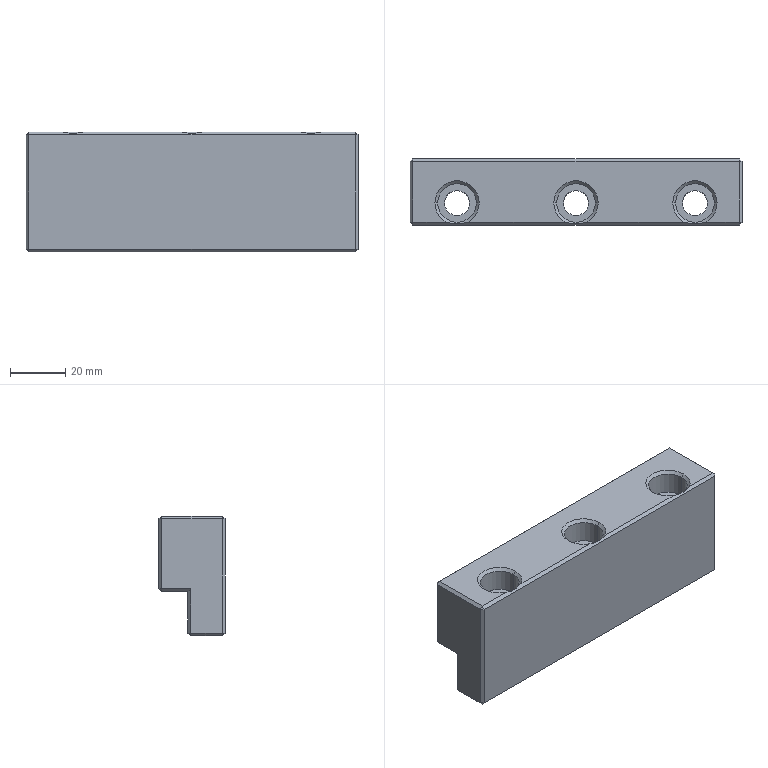Part | Creo | 1 solid | 56 faces | box 120 x 24 x 43.328 mm | volume 93421 mm3 | plane 38 | cylinder 12 | cone 6 | commonest cylinder face diameters 9 x6 14 x6
STEP:
#1=CARTESIAN_POINT('',(0.,0.,0.));
#2=DIRECTION('',(0.,0.,1.));
#3=DIRECTION('',(1.,0.,0.));
#4=AXIS2_PLACEMENT_3D('',#1,#2,#3);
#5=CARTESIAN_POINT('',(81.,-133.9,-32.828));
#6=VERTEX_POINT('',#5);
#7=CARTESIAN_POINT('',(81.,-133.9,8.5));
#8=VERTEX_POINT('',#7);
#9=CARTESIAN_POINT('',(81.,-133.9,-32.828));
#10=DIRECTION('',(0.,0.,1.));
#11=VECTOR('',#10,41.328);
#12=LINE('',#9,#11);
#13=EDGE_CURVE('',#6,#8,#12,.T.);
#14=ORIENTED_EDGE('',*,*,#13,.T.);
#15=CARTESIAN_POINT('',(199.,-133.9,8.5));
#16=VERTEX_POINT('',#15);
#17=CARTESIAN_POINT('',(81.,-133.9,8.5));
#18=DIRECTION('',(1.,0.,0.));
#19=VECTOR('',#18,118.);
#20=LINE('',#17,#19);
#21=EDGE_CURVE('',#8,#16,#20,.T.);
#22=ORIENTED_EDGE('',*,*,#21,.T.);
#23=CARTESIAN_POINT('',(199.,-133.9,-32.828));
#24=VERTEX_POINT('',#23);
#25=CARTESIAN_POINT('',(199.,-133.9,8.5));
#26=DIRECTION('',(0.,0.,-1.));
#27=VECTOR('',#26,41.328);
#28=LINE('',#25,#27);
#29=EDGE_CURVE('',#16,#24,#28,.T.);
#30=ORIENTED_EDGE('',*,*,#29,.T.);
#31=CARTESIAN_POINT('',(199.,-133.9,-32.828));
#32=DIRECTION('',(-1.,0.,0.));
#33=VECTOR('',#32,118.);
#34=LINE('',#31,#33);
#35=EDGE_CURVE('',#24,#6,#34,.T.);
#36=ORIENTED_EDGE('',*,*,#35,.T.);
#37=EDGE_LOOP('',(#14,#22,#30,#36));
#38=FACE_OUTER_BOUND('',#37,.F.);
#39=CARTESIAN_POINT('',(230.,-133.9,22.172));
#40=DIRECTION('',(0.,1.,0.));
#41=DIRECTION('',(0.,0.,-1.));
#42=AXIS2_PLACEMENT_3D('',#39,#40,#41);
#43=PLANE('',#42);
#44=ADVANCED_FACE('',(#38),#43,.F.);
#45=CARTESIAN_POINT('',(80.,-132.9,8.5));
#46=VERTEX_POINT('',#45);
#47=CARTESIAN_POINT('',(80.,-132.9,8.5));
#48=DIRECTION('',(0.7071,-0.7071,0.));
#49=VECTOR('',#48,1.414);
#50=LINE('',#47,#49);
#51=EDGE_CURVE('',#46,#8,#50,.T.);
#52=ORIENTED_EDGE('',*,*,#51,.T.);
#53=ORIENTED_EDGE('',*,*,#13,.F.);
#54=CARTESIAN_POINT('',(80.,-132.9,-32.828));
#55=VERTEX_POINT('',#54);
#56=CARTESIAN_POINT('',(81.,-133.9,-32.828));
#57=DIRECTION('',(-0.7071,0.7071,0.));
#58=VECTOR('',#57,1.414);
#59=LINE('',#56,#58);
#60=EDGE_CURVE('',#6,#55,#59,.T.);
#61=ORIENTED_EDGE('',*,*,#60,.T.);
#62=CARTESIAN_POINT('',(80.,-132.9,8.5));
#63=DIRECTION('',(0.,0.,-1.));
#64=VECTOR('',#63,41.328);
#65=LINE('',#62,#64);
#66=EDGE_CURVE('',#46,#55,#65,.T.);
#67=ORIENTED_EDGE('',*,*,#66,.F.);
#68=EDGE_LOOP('',(#52,#53,#61,#67));
#69=FACE_OUTER_BOUND('',#68,.F.);
#70=CARTESIAN_POINT('',(81.,-133.9,22.172));
#71=DIRECTION('',(0.7071,0.7071,0.));
#72=DIRECTION('',(0.,0.,-1.));
#73=AXIS2_PLACEMENT_3D('',#70,#71,#72);
#74=PLANE('',#73);
#75=ADVANCED_FACE('',(#69),#74,.F.);
#76=CARTESIAN_POINT('',(81.,-132.9,9.5));
#77=VERTEX_POINT('',#76);
#78=CARTESIAN_POINT('',(81.,-133.9,8.5));
#79=DIRECTION('',(0.,0.7071,0.7071));
#80=VECTOR('',#79,1.414);
#81=LINE('',#78,#80);
#82=EDGE_CURVE('',#8,#77,#81,.T.);
#83=ORIENTED_EDGE('',*,*,#82,.F.);
#84=ORIENTED_EDGE('',*,*,#51,.F.);
#85=CARTESIAN_POINT('',(80.,-132.9,8.5));
#86=DIRECTION('',(0.7071,0.,0.7071));
#87=VECTOR('',#86,1.414);
#88=LINE('',#85,#87);
#89=EDGE_CURVE('',#46,#77,#88,.T.);
#90=ORIENTED_EDGE('',*,*,#89,.T.);
#91=EDGE_LOOP('',(#83,#84,#90));
#92=FACE_OUTER_BOUND('',#91,.F.);
#93=CARTESIAN_POINT('',(81.,-132.9,9.5));
#94=DIRECTION('',(-0.5774,-0.5774,0.5774));
#95=DIRECTION('',(0.7071,0.,0.7071));
#96=AXIS2_PLACEMENT_3D('',#93,#94,#95);
#97=PLANE('',#96);
#98=ADVANCED_FACE('',(#92),#97,.T.);
#99=CARTESIAN_POINT('',(199.,-132.9,9.5));
#100=VERTEX_POINT('',#99);
#101=CARTESIAN_POINT('',(199.,-133.9,8.5));
#102=DIRECTION('',(0.,0.7071,0.7071));
#103=VECTOR('',#102,1.414);
#104=LINE('',#101,#103);
#105=EDGE_CURVE('',#16,#100,#104,.T.);
#106=ORIENTED_EDGE('',*,*,#105,.F.);
#107=ORIENTED_EDGE('',*,*,#21,.F.);
#108=ORIENTED_EDGE('',*,*,#82,.T.);
#109=CARTESIAN_POINT('',(93.127,-132.9,9.5));
#110=VERTEX_POINT('',#109);
#111=CARTESIAN_POINT('',(93.127,-132.9,9.5));
#112=DIRECTION('',(-1.,0.,0.));
#113=VECTOR('',#112,12.127);
#114=LINE('',#111,#113);
#115=EDGE_CURVE('',#110,#77,#114,.T.);
#116=ORIENTED_EDGE('',*,*,#115,.F.);
#117=CARTESIAN_POINT('',(100.873,-132.9,9.5));
#118=VERTEX_POINT('',#117);
#119=CARTESIAN_POINT('',(93.127,-132.9,9.5));
#120=CARTESIAN_POINT('',(93.752,-133.061,9.339));
#121=CARTESIAN_POINT('',(95.017,-133.311,9.089));
#122=CARTESIAN_POINT('',(97.,-133.445,8.955));
#123=CARTESIAN_POINT('',(98.983,-133.311,9.089));
#124=CARTESIAN_POINT('',(100.248,-133.061,9.339));
#125=CARTESIAN_POINT('',(100.873,-132.9,9.5));
#126=B_SPLINE_CURVE_WITH_KNOTS('',3,(#119,#120,#121,#122,#123,#124,#125),.UNSPECIFIED.,.F.,.F.,(4,1,1,1,4),(0.,0.25,0.5,0.75,1.),.UNSPECIFIED.);
#127=EDGE_CURVE('',#110,#118,#126,.T.);
#128=ORIENTED_EDGE('',*,*,#127,.T.);
#129=CARTESIAN_POINT('',(136.127,-132.9,9.5));
#130=VERTEX_POINT('',#129);
#131=CARTESIAN_POINT('',(136.127,-132.9,9.5));
#132=DIRECTION('',(-1.,0.,0.));
#133=VECTOR('',#132,35.254);
#134=LINE('',#131,#133);
#135=EDGE_CURVE('',#130,#118,#134,.T.);
#136=ORIENTED_EDGE('',*,*,#135,.F.);
#137=CARTESIAN_POINT('',(143.873,-132.9,9.5));
#138=VERTEX_POINT('',#137);
#139=CARTESIAN_POINT('',(136.127,-132.9,9.5));
#140=CARTESIAN_POINT('',(136.752,-133.061,9.339));
#141=CARTESIAN_POINT('',(138.017,-133.311,9.089));
#142=CARTESIAN_POINT('',(140.,-133.445,8.955));
#143=CARTESIAN_POINT('',(141.983,-133.311,9.089));
#144=CARTESIAN_POINT('',(143.248,-133.061,9.339));
#145=CARTESIAN_POINT('',(143.873,-132.9,9.5));
#146=B_SPLINE_CURVE_WITH_KNOTS('',3,(#139,#140,#141,#142,#143,#144,#145),.UNSPECIFIED.,.F.,.F.,(4,1,1,1,4),(0.,0.25,0.5,0.75,1.),.UNSPECIFIED.);
#147=EDGE_CURVE('',#130,#138,#146,.T.);
#148=ORIENTED_EDGE('',*,*,#147,.T.);
#149=CARTESIAN_POINT('',(179.127,-132.9,9.5));
#150=VERTEX_POINT('',#149);
#151=CARTESIAN_POINT('',(179.127,-132.9,9.5));
#152=DIRECTION('',(-1.,0.,0.));
#153=VECTOR('',#152,35.254);
#154=LINE('',#151,#153);
#155=EDGE_CURVE('',#150,#138,#154,.T.);
#156=ORIENTED_EDGE('',*,*,#155,.F.);
#157=CARTESIAN_POINT('',(186.873,-132.9,9.5));
#158=VERTEX_POINT('',#157);
#159=CARTESIAN_POINT('',(179.127,-132.9,9.5));
#160=CARTESIAN_POINT('',(179.752,-133.061,9.339));
#161=CARTESIAN_POINT('',(181.017,-133.311,9.089));
#162=CARTESIAN_POINT('',(183.,-133.445,8.955));
#163=CARTESIAN_POINT('',(184.983,-133.311,9.089));
#164=CARTESIAN_POINT('',(186.248,-133.061,9.339));
#165=CARTESIAN_POINT('',(186.873,-132.9,9.5));
#166=B_SPLINE_CURVE_WITH_KNOTS('',3,(#159,#160,#161,#162,#163,#164,#165),.UNSPECIFIED.,.F.,.F.,(4,1,1,1,4),(0.,0.25,0.5,0.75,1.),.UNSPECIFIED.);
#167=EDGE_CURVE('',#150,#158,#166,.T.);
#168=ORIENTED_EDGE('',*,*,#167,.T.);
#169=CARTESIAN_POINT('',(199.,-132.9,9.5));
#170=DIRECTION('',(-1.,0.,0.));
#171=VECTOR('',#170,12.127);
#172=LINE('',#169,#171);
#173=EDGE_CURVE('',#100,#158,#172,.T.);
#174=ORIENTED_EDGE('',*,*,#173,.F.);
#175=EDGE_LOOP('',(#106,#107,#108,#116,#128,#136,#148,#156,#168,#174));
#176=FACE_OUTER_BOUND('',#175,.F.);
#177=CARTESIAN_POINT('',(230.,-133.9,8.5));
#178=DIRECTION('',(0.,-0.7071,0.7071));
#179=DIRECTION('',(1.,0.,0.));
#180=AXIS2_PLACEMENT_3D('',#177,#178,#179);
#181=PLANE('',#180);
#182=ADVANCED_FACE('',(#176),#181,.T.);
#183=CARTESIAN_POINT('',(200.,-132.9,8.5));
#184=VERTEX_POINT('',#183);
#185=CARTESIAN_POINT('',(200.,-132.9,8.5));
#186=DIRECTION('',(-0.7071,0.,0.7071));
#187=VECTOR('',#186,1.414);
#188=LINE('',#185,#187);
#189=EDGE_CURVE('',#184,#100,#188,.T.);
#190=ORIENTED_EDGE('',*,*,#189,.F.);
#191=CARTESIAN_POINT('',(199.,-133.9,8.5));
#192=DIRECTION('',(0.7071,0.7071,0.));
#193=VECTOR('',#192,1.414);
#194=LINE('',#191,#193);
#195=EDGE_CURVE('',#16,#184,#194,.T.);
#196=ORIENTED_EDGE('',*,*,#195,.F.);
#197=ORIENTED_EDGE('',*,*,#105,.T.);
#198=EDGE_LOOP('',(#190,#196,#197));
#199=FACE_OUTER_BOUND('',#198,.F.);
#200=CARTESIAN_POINT('',(199.,-133.9,8.5));
#201=DIRECTION('',(0.5774,-0.5774,0.5774));
#202=DIRECTION('',(0.,-0.7071,-0.7071));
#203=AXIS2_PLACEMENT_3D('',#200,#201,#202);
#204=PLANE('',#203);
#205=ADVANCED_FACE('',(#199),#204,.T.);
#206=CARTESIAN_POINT('',(199.,-110.9,9.5));
#207=VERTEX_POINT('',#206);
#208=CARTESIAN_POINT('',(200.,-110.9,8.5));
#209=VERTEX_POINT('',#208);
#210=CARTESIAN_POINT('',(199.,-110.9,9.5));
#211=DIRECTION('',(0.7071,0.,-0.7071));
#212=VECTOR('',#211,1.414);
#213=LINE('',#210,#212);
#214=EDGE_CURVE('',#207,#209,#213,.T.);
#215=ORIENTED_EDGE('',*,*,#214,.T.);
#216=CARTESIAN_POINT('',(200.,-132.9,8.5));
#217=DIRECTION('',(0.,1.,0.));
#218=VECTOR('',#217,22.);
#219=LINE('',#216,#218);
#220=EDGE_CURVE('',#184,#209,#219,.T.);
#221=ORIENTED_EDGE('',*,*,#220,.F.);
#222=ORIENTED_EDGE('',*,*,#189,.T.);
#223=CARTESIAN_POINT('',(199.,-110.9,9.5));
#224=DIRECTION('',(0.,-1.,0.));
#225=VECTOR('',#224,22.);
#226=LINE('',#223,#225);
#227=EDGE_CURVE('',#207,#100,#226,.T.);
#228=ORIENTED_EDGE('',*,*,#227,.F.);
#229=EDGE_LOOP('',(#215,#221,#222,#228));
#230=FACE_OUTER_BOUND('',#229,.F.);
#231=CARTESIAN_POINT('',(199.,-0.8,9.5));
#232=DIRECTION('',(-0.7071,0.,-0.7071));
#233=DIRECTION('',(0.,1.,0.));
#234=AXIS2_PLACEMENT_3D('',#231,#232,#233);
#235=PLANE('',#234);
#236=ADVANCED_FACE('',(#230),#235,.F.);
#237=CARTESIAN_POINT('',(199.,-109.9,8.5));
#238=VERTEX_POINT('',#237);
#239=CARTESIAN_POINT('',(200.,-110.9,8.5));
#240=DIRECTION('',(-0.7071,0.7071,0.));
#241=VECTOR('',#240,1.414);
#242=LINE('',#239,#241);
#243=EDGE_CURVE('',#209,#238,#242,.T.);
#244=ORIENTED_EDGE('',*,*,#243,.F.);
#245=ORIENTED_EDGE('',*,*,#214,.F.);
#246=CARTESIAN_POINT('',(199.,-110.9,9.5));
#247=DIRECTION('',(0.,0.7071,-0.7071));
#248=VECTOR('',#247,1.414);
#249=LINE('',#246,#248);
#250=EDGE_CURVE('',#207,#238,#249,.T.);
#251=ORIENTED_EDGE('',*,*,#250,.T.);
#252=EDGE_LOOP('',(#244,#245,#251));
#253=FACE_OUTER_BOUND('',#252,.F.);
#254=CARTESIAN_POINT('',(200.,-110.9,8.5));
#255=DIRECTION('',(0.5774,0.5774,0.5774));
#256=DIRECTION('',(0.,-0.7071,0.7071));
#257=AXIS2_PLACEMENT_3D('',#254,#255,#256);
#258=PLANE('',#257);
#259=ADVANCED_FACE('',(#253),#258,.T.);
#260=CARTESIAN_POINT('',(199.,-109.9,-16.828));
#261=VERTEX_POINT('',#260);
#262=CARTESIAN_POINT('',(200.,-110.9,-16.828));
#263=VERTEX_POINT('',#262);
#264=CARTESIAN_POINT('',(199.,-109.9,-16.828));
#265=DIRECTION('',(0.7071,-0.7071,0.));
#266=VECTOR('',#265,1.414);
#267=LINE('',#264,#266);
#268=EDGE_CURVE('',#261,#263,#267,.T.);
#269=ORIENTED_EDGE('',*,*,#268,.T.);
#270=CARTESIAN_POINT('',(200.,-110.9,8.5));
#271=DIRECTION('',(0.,0.,-1.));
#272=VECTOR('',#271,25.328);
#273=LINE('',#270,#272);
#274=EDGE_CURVE('',#209,#263,#273,.T.);
#275=ORIENTED_EDGE('',*,*,#274,.F.);
#276=ORIENTED_EDGE('',*,*,#243,.T.);
#277=CARTESIAN_POINT('',(199.,-109.9,-16.828));
#278=DIRECTION('',(0.,0.,1.));
#279=VECTOR('',#278,25.328);
#280=LINE('',#277,#279);
#281=EDGE_CURVE('',#261,#238,#280,.T.);
#282=ORIENTED_EDGE('',*,*,#281,.F.);
#283=EDGE_LOOP('',(#269,#275,#276,#282));
#284=FACE_OUTER_BOUND('',#283,.F.);
#285=CARTESIAN_POINT('',(199.,-109.9,-15.828));
#286=DIRECTION('',(0.7071,0.7071,0.));
#287=DIRECTION('',(0.,0.,1.));
#288=AXIS2_PLACEMENT_3D('',#285,#286,#287);
#289=PLANE('',#288);
#290=ADVANCED_FACE('',(#284),#289,.T.);
#291=CARTESIAN_POINT('',(199.,-110.9,-17.828));
#292=VERTEX_POINT('',#291);
#293=CARTESIAN_POINT('',(199.,-110.9,-17.828));
#294=DIRECTION('',(0.,0.7071,0.7071));
#295=VECTOR('',#294,1.414);
#296=LINE('',#293,#295);
#297=EDGE_CURVE('',#292,#261,#296,.T.);
#298=ORIENTED_EDGE('',*,*,#297,.F.);
#299=CARTESIAN_POINT('',(200.,-110.9,-16.828));
#300=DIRECTION('',(-0.7071,0.,-0.7071));
#301=VECTOR('',#300,1.414);
#302=LINE('',#299,#301);
#303=EDGE_CURVE('',#263,#292,#302,.T.);
#304=ORIENTED_EDGE('',*,*,#303,.F.);
#305=ORIENTED_EDGE('',*,*,#268,.F.);
#306=EDGE_LOOP('',(#298,#304,#305));
#307=FACE_OUTER_BOUND('',#306,.F.);
#308=CARTESIAN_POINT('',(199.,-110.9,-17.828));
#309=DIRECTION('',(0.5774,0.5774,-0.5774));
#310=DIRECTION('',(-0.7071,0.,-0.7071));
#311=AXIS2_PLACEMENT_3D('',#308,#309,#310);
#312=PLANE('',#311);
#313=ADVANCED_FACE('',(#307),#312,.T.);
#314=CARTESIAN_POINT('',(81.,-109.9,-16.828));
#315=VERTEX_POINT('',#314);
#316=CARTESIAN_POINT('',(81.,-110.9,-17.828));
#317=VERTEX_POINT('',#316);
#318=CARTESIAN_POINT('',(81.,-109.9,-16.828));
#319=DIRECTION('',(0.,-0.7071,-0.7071));
#320=VECTOR('',#319,1.414);
#321=LINE('',#318,#320);
#322=EDGE_CURVE('',#315,#317,#321,.T.);
#323=ORIENTED_EDGE('',*,*,#322,.T.);
#324=CARTESIAN_POINT('',(199.,-110.9,-17.828));
#325=DIRECTION('',(-1.,0.,0.));
#326=VECTOR('',#325,118.);
#327=LINE('',#324,#326);
#328=EDGE_CURVE('',#292,#317,#327,.T.);
#329=ORIENTED_EDGE('',*,*,#328,.F.);
#330=ORIENTED_EDGE('',*,*,#297,.T.);
#331=CARTESIAN_POINT('',(81.,-109.9,-16.828));
#332=DIRECTION('',(1.,0.,0.));
#333=VECTOR('',#332,118.);
#334=LINE('',#331,#333);
#335=EDGE_CURVE('',#315,#261,#334,.T.);
#336=ORIENTED_EDGE('',*,*,#335,.F.);
#337=EDGE_LOOP('',(#323,#329,#330,#336));
#338=FACE_OUTER_BOUND('',#337,.F.);
#339=CARTESIAN_POINT('',(230.,-109.9,-16.828));
#340=DIRECTION('',(0.,-0.7071,0.7071));
#341=DIRECTION('',(-1.,0.,0.));
#342=AXIS2_PLACEMENT_3D('',#339,#340,#341);
#343=PLANE('',#342);
#344=ADVANCED_FACE('',(#338),#343,.F.);
#345=CARTESIAN_POINT('',(80.,-110.9,-16.828));
#346=VERTEX_POINT('',#345);
#347=CARTESIAN_POINT('',(81.,-110.9,-17.828));
#348=DIRECTION('',(-0.7071,0.,0.7071));
#349=VECTOR('',#348,1.414);
#350=LINE('',#347,#349);
#351=EDGE_CURVE('',#317,#346,#350,.T.);
#352=ORIENTED_EDGE('',*,*,#351,.F.);
#353=ORIENTED_EDGE('',*,*,#322,.F.);
#354=CARTESIAN_POINT('',(80.,-110.9,-16.828));
#355=DIRECTION('',(0.7071,0.7071,0.));
#356=VECTOR('',#355,1.414);
#357=LINE('',#354,#356);
#358=EDGE_CURVE('',#346,#315,#357,.T.);
#359=ORIENTED_EDGE('',*,*,#358,.F.);
#360=EDGE_LOOP('',(#352,#353,#359));
#361=FACE_OUTER_BOUND('',#360,.F.);
#362=CARTESIAN_POINT('',(80.,-110.9,-16.828));
#363=DIRECTION('',(-0.5774,0.5774,-0.5774));
#364=DIRECTION('',(-0.7071,0.,0.7071));
#365=AXIS2_PLACEMENT_3D('',#362,#363,#364);
#366=PLANE('',#365);
#367=ADVANCED_FACE('',(#361),#366,.T.);
#368=ORIENTED_EDGE('',*,*,#351,.T.);
#369=CARTESIAN_POINT('',(80.,-121.4,-16.828));
#370=VERTEX_POINT('',#369);
#371=CARTESIAN_POINT('',(80.,-121.4,-16.828));
#372=DIRECTION('',(0.,1.,0.));
#373=VECTOR('',#372,10.5);
#374=LINE('',#371,#373);
#375=EDGE_CURVE('',#370,#346,#374,.T.);
#376=ORIENTED_EDGE('',*,*,#375,.F.);
#377=CARTESIAN_POINT('',(81.,-120.4,-17.828));
#378=VERTEX_POINT('',#377);
#379=CARTESIAN_POINT('',(81.,-120.4,-17.828));
#380=DIRECTION('',(-0.5774,-0.5774,0.5774));
#381=VECTOR('',#380,1.732);
#382=LINE('',#379,#381);
#383=EDGE_CURVE('',#378,#370,#382,.T.);
#384=ORIENTED_EDGE('',*,*,#383,.F.);
#385=CARTESIAN_POINT('',(81.,-110.9,-17.828));
#386=DIRECTION('',(0.,-1.,0.));
#387=VECTOR('',#386,9.5);
#388=LINE('',#385,#387);
#389=EDGE_CURVE('',#317,#378,#388,.T.);
#390=ORIENTED_EDGE('',*,*,#389,.F.);
#391=EDGE_LOOP('',(#368,#376,#384,#390));
#392=FACE_OUTER_BOUND('',#391,.F.);
#393=CARTESIAN_POINT('',(80.,-133.9,-16.828));
#394=DIRECTION('',(0.7071,0.,0.7071));
#395=DIRECTION('',(0.,-1.,0.));
#396=AXIS2_PLACEMENT_3D('',#393,#394,#395);
#397=PLANE('',#396);
#398=ADVANCED_FACE('',(#392),#397,.F.);
#399=ORIENTED_EDGE('',*,*,#66,.T.);
#400=CARTESIAN_POINT('',(80.,-121.4,-32.828));
#401=VERTEX_POINT('',#400);
#402=CARTESIAN_POINT('',(80.,-132.9,-32.828));
#403=DIRECTION('',(0.,1.,0.));
#404=VECTOR('',#403,11.5);
#405=LINE('',#402,#404);
#406=EDGE_CURVE('',#55,#401,#405,.T.);
#407=ORIENTED_EDGE('',*,*,#406,.T.);
#408=CARTESIAN_POINT('',(80.,-121.4,-32.828));
#409=DIRECTION('',(0.,0.,1.));
#410=VECTOR('',#409,16.);
#411=LINE('',#408,#410);
#412=EDGE_CURVE('',#401,#370,#411,.T.);
#413=ORIENTED_EDGE('',*,*,#412,.T.);
#414=ORIENTED_EDGE('',*,*,#375,.T.);
#415=CARTESIAN_POINT('',(80.,-110.9,8.5));
#416=VERTEX_POINT('',#415);
#417=CARTESIAN_POINT('',(80.,-110.9,-16.828));
#418=DIRECTION('',(0.,0.,1.));
#419=VECTOR('',#418,25.328);
#420=LINE('',#417,#419);
#421=EDGE_CURVE('',#346,#416,#420,.T.);
#422=ORIENTED_EDGE('',*,*,#421,.T.);
#423=CARTESIAN_POINT('',(80.,-110.9,8.5));
#424=DIRECTION('',(0.,-1.,0.));
#425=VECTOR('',#424,22.);
#426=LINE('',#423,#425);
#427=EDGE_CURVE('',#416,#46,#426,.T.);
#428=ORIENTED_EDGE('',*,*,#427,.T.);
#429=EDGE_LOOP('',(#399,#407,#413,#414,#422,#428));
#430=FACE_OUTER_BOUND('',#429,.F.);
#431=CARTESIAN_POINT('',(80.,-133.9,22.172));
#432=DIRECTION('',(1.,0.,0.));
#433=DIRECTION('',(0.,0.,-1.));
#434=AXIS2_PLACEMENT_3D('',#431,#432,#433);
#435=PLANE('',#434);
#436=ADVANCED_FACE('',(#430),#435,.F.);
#437=CARTESIAN_POINT('',(81.,-121.4,-33.828));
#438=VERTEX_POINT('',#437);
#439=CARTESIAN_POINT('',(81.,-121.4,-33.828));
#440=DIRECTION('',(-0.7071,0.,0.7071));
#441=VECTOR('',#440,1.414);
#442=LINE('',#439,#441);
#443=EDGE_CURVE('',#438,#401,#442,.T.);
#444=ORIENTED_EDGE('',*,*,#443,.T.);
#445=ORIENTED_EDGE('',*,*,#406,.F.);
#446=CARTESIAN_POINT('',(81.,-132.9,-33.828));
#447=VERTEX_POINT('',#446);
#448=CARTESIAN_POINT('',(81.,-132.9,-33.828));
#449=DIRECTION('',(-0.7071,0.,0.7071));
#450=VECTOR('',#449,1.414);
#451=LINE('',#448,#450);
#452=EDGE_CURVE('',#447,#55,#451,.T.);
#453=ORIENTED_EDGE('',*,*,#452,.F.);
#454=CARTESIAN_POINT('',(81.,-121.4,-33.828));
#455=DIRECTION('',(0.,-1.,0.));
#456=VECTOR('',#455,11.5);
#457=LINE('',#454,#456);
#458=EDGE_CURVE('',#438,#447,#457,.T.);
#459=ORIENTED_EDGE('',*,*,#458,.F.);
#460=EDGE_LOOP('',(#444,#445,#453,#459));
#461=FACE_OUTER_BOUND('',#460,.F.);
#462=CARTESIAN_POINT('',(81.,-133.9,-33.828));
#463=DIRECTION('',(0.7071,0.,0.7071));
#464=DIRECTION('',(0.,1.,0.));
#465=AXIS2_PLACEMENT_3D('',#462,#463,#464);
#466=PLANE('',#465);
#467=ADVANCED_FACE('',(#461),#466,.F.);
#468=CARTESIAN_POINT('',(81.,-120.4,-32.828));
#469=VERTEX_POINT('',#468);
#470=CARTESIAN_POINT('',(80.,-121.4,-32.828));
#471=DIRECTION('',(0.7071,0.7071,0.));
#472=VECTOR('',#471,1.414);
#473=LINE('',#470,#472);
#474=EDGE_CURVE('',#401,#469,#473,.T.);
#475=ORIENTED_EDGE('',*,*,#474,.F.);
#476=ORIENTED_EDGE('',*,*,#443,.F.);
#477=CARTESIAN_POINT('',(81.,-120.4,-32.828));
#478=DIRECTION('',(0.,-0.7071,-0.7071));
#479=VECTOR('',#478,1.414);
#480=LINE('',#477,#479);
#481=EDGE_CURVE('',#469,#438,#480,.T.);
#482=ORIENTED_EDGE('',*,*,#481,.F.);
#483=EDGE_LOOP('',(#475,#476,#482));
#484=FACE_OUTER_BOUND('',#483,.F.);
#485=CARTESIAN_POINT('',(81.,-120.4,-32.828));
#486=DIRECTION('',(-0.5774,0.5774,-0.5774));
#487=DIRECTION('',(-0.7071,0.,0.7071));
#488=AXIS2_PLACEMENT_3D('',#485,#486,#487);
#489=PLANE('',#488);
#490=ADVANCED_FACE('',(#484),#489,.T.);
#491=ORIENTED_EDGE('',*,*,#383,.T.);
#492=ORIENTED_EDGE('',*,*,#412,.F.);
#493=ORIENTED_EDGE('',*,*,#474,.T.);
#494=CARTESIAN_POINT('',(81.,-120.4,-17.828));
#495=DIRECTION('',(0.,0.,-1.));
#496=VECTOR('',#495,15.);
#497=LINE('',#494,#496);
#498=EDGE_CURVE('',#378,#469,#497,.T.);
#499=ORIENTED_EDGE('',*,*,#498,.F.);
#500=EDGE_LOOP('',(#491,#492,#493,#499));
#501=FACE_OUTER_BOUND('',#500,.F.);
#502=CARTESIAN_POINT('',(81.,-120.4,-33.828));
#503=DIRECTION('',(0.7071,-0.7071,0.));
#504=DIRECTION('',(0.,0.,1.));
#505=AXIS2_PLACEMENT_3D('',#502,#503,#504);
#506=PLANE('',#505);
#507=ADVANCED_FACE('',(#501),#506,.F.);
#508=CARTESIAN_POINT('',(199.,-120.4,-17.828));
#509=VERTEX_POINT('',#508);
#510=CARTESIAN_POINT('',(81.,-120.4,-17.828));
#511=DIRECTION('',(1.,0.,0.));
#512=VECTOR('',#511,118.);
#513=LINE('',#510,#512);
#514=EDGE_CURVE('',#378,#509,#513,.T.);
#515=ORIENTED_EDGE('',*,*,#514,.F.);
#516=ORIENTED_EDGE('',*,*,#498,.T.);
#517=CARTESIAN_POINT('',(199.,-120.4,-32.828));
#518=VERTEX_POINT('',#517);
#519=CARTESIAN_POINT('',(81.,-120.4,-32.828));
#520=DIRECTION('',(1.,0.,0.));
#521=VECTOR('',#520,118.);
#522=LINE('',#519,#521);
#523=EDGE_CURVE('',#469,#518,#522,.T.);
#524=ORIENTED_EDGE('',*,*,#523,.T.);
#525=CARTESIAN_POINT('',(199.,-120.4,-32.828));
#526=DIRECTION('',(0.,0.,1.));
#527=VECTOR('',#526,15.);
#528=LINE('',#525,#527);
#529=EDGE_CURVE('',#518,#509,#528,.T.);
#530=ORIENTED_EDGE('',*,*,#529,.T.);
#531=EDGE_LOOP('',(#515,#516,#524,#530));
#532=FACE_OUTER_BOUND('',#531,.F.);
#533=CARTESIAN_POINT('',(230.,-120.4,-33.828));
#534=DIRECTION('',(0.,-1.,0.));
#535=DIRECTION('',(0.,0.,1.));
#536=AXIS2_PLACEMENT_3D('',#533,#534,#535);
#537=PLANE('',#536);
#538=ADVANCED_FACE('',(#532),#537,.F.);
#539=ORIENTED_EDGE('',*,*,#328,.T.);
#540=ORIENTED_EDGE('',*,*,#389,.T.);
#541=ORIENTED_EDGE('',*,*,#514,.T.);
#542=CARTESIAN_POINT('',(199.,-120.4,-17.828));
#543=DIRECTION('',(0.,1.,0.));
#544=VECTOR('',#543,9.5);
#545=LINE('',#542,#544);
#546=EDGE_CURVE('',#509,#292,#545,.T.);
#547=ORIENTED_EDGE('',*,*,#546,.T.);
#548=EDGE_LOOP('',(#539,#540,#541,#547));
#549=FACE_OUTER_BOUND('',#548,.F.);
#550=CARTESIAN_POINT('',(230.,-120.4,-17.828));
#551=DIRECTION('',(0.,0.,1.));
#552=DIRECTION('',(0.,1.,0.));
#553=AXIS2_PLACEMENT_3D('',#550,#551,#552);
#554=PLANE('',#553);
#555=ADVANCED_FACE('',(#549),#554,.F.);
#556=ORIENTED_EDGE('',*,*,#303,.T.);
#557=ORIENTED_EDGE('',*,*,#546,.F.);
#558=CARTESIAN_POINT('',(200.,-121.4,-16.828));
#559=VERTEX_POINT('',#558);
#560=CARTESIAN_POINT('',(200.,-121.4,-16.828));
#561=DIRECTION('',(-0.5774,0.5774,-0.5774));
#562=VECTOR('',#561,1.732);
#563=LINE('',#560,#562);
#564=EDGE_CURVE('',#559,#509,#563,.T.);
#565=ORIENTED_EDGE('',*,*,#564,.F.);
#566=CARTESIAN_POINT('',(200.,-110.9,-16.828));
#567=DIRECTION('',(0.,-1.,0.));
#568=VECTOR('',#567,10.5);
#569=LINE('',#566,#568);
#570=EDGE_CURVE('',#263,#559,#569,.T.);
#571=ORIENTED_EDGE('',*,*,#570,.F.);
#572=EDGE_LOOP('',(#556,#557,#565,#571));
#573=FACE_OUTER_BOUND('',#572,.F.);
#574=CARTESIAN_POINT('',(199.,-120.4,-17.828));
#575=DIRECTION('',(0.7071,0.,-0.7071));
#576=DIRECTION('',(0.,1.,0.));
#577=AXIS2_PLACEMENT_3D('',#574,#575,#576);
#578=PLANE('',#577);
#579=ADVANCED_FACE('',(#573),#578,.T.);
#580=ORIENTED_EDGE('',*,*,#564,.T.);
#581=ORIENTED_EDGE('',*,*,#529,.F.);
#582=CARTESIAN_POINT('',(200.,-121.4,-32.828));
#583=VERTEX_POINT('',#582);
#584=CARTESIAN_POINT('',(199.,-120.4,-32.828));
#585=DIRECTION('',(0.7071,-0.7071,0.));
#586=VECTOR('',#585,1.414);
#587=LINE('',#584,#586);
#588=EDGE_CURVE('',#518,#583,#587,.T.);
#589=ORIENTED_EDGE('',*,*,#588,.T.);
#590=CARTESIAN_POINT('',(200.,-121.4,-16.828));
#591=DIRECTION('',(0.,0.,-1.));
#592=VECTOR('',#591,16.);
#593=LINE('',#590,#592);
#594=EDGE_CURVE('',#559,#583,#593,.T.);
#595=ORIENTED_EDGE('',*,*,#594,.F.);
#596=EDGE_LOOP('',(#580,#581,#589,#595));
#597=FACE_OUTER_BOUND('',#596,.F.);
#598=CARTESIAN_POINT('',(199.,-120.4,-33.828));
#599=DIRECTION('',(0.7071,0.7071,0.));
#600=DIRECTION('',(0.,0.,1.));
#601=AXIS2_PLACEMENT_3D('',#598,#599,#600);
#602=PLANE('',#601);
#603=ADVANCED_FACE('',(#597),#602,.T.);
#604=CARTESIAN_POINT('',(199.,-121.4,-33.828));
#605=VERTEX_POINT('',#604);
#606=CARTESIAN_POINT('',(199.,-121.4,-33.828));
#607=DIRECTION('',(0.,0.7071,0.7071));
#608=VECTOR('',#607,1.414);
#609=LINE('',#606,#608);
#610=EDGE_CURVE('',#605,#518,#609,.T.);
#611=ORIENTED_EDGE('',*,*,#610,.F.);
#612=CARTESIAN_POINT('',(200.,-121.4,-32.828));
#613=DIRECTION('',(-0.7071,0.,-0.7071));
#614=VECTOR('',#613,1.414);
#615=LINE('',#612,#614);
#616=EDGE_CURVE('',#583,#605,#615,.T.);
#617=ORIENTED_EDGE('',*,*,#616,.F.);
#618=ORIENTED_EDGE('',*,*,#588,.F.);
#619=EDGE_LOOP('',(#611,#617,#618));
#620=FACE_OUTER_BOUND('',#619,.F.);
#621=CARTESIAN_POINT('',(199.,-121.4,-33.828));
#622=DIRECTION('',(0.5774,0.5774,-0.5774));
#623=DIRECTION('',(-0.7071,0.,-0.7071));
#624=AXIS2_PLACEMENT_3D('',#621,#622,#623);
#625=PLANE('',#624);
#626=ADVANCED_FACE('',(#620),#625,.T.);
#627=ORIENTED_EDGE('',*,*,#481,.T.);
#628=CARTESIAN_POINT('',(97.,-121.4,-33.828));
#629=VERTEX_POINT('',#628);
#630=CARTESIAN_POINT('',(97.,-121.4,-33.828));
#631=DIRECTION('',(-1.,0.,0.));
#632=VECTOR('',#631,16.);
#633=LINE('',#630,#632);
#634=EDGE_CURVE('',#629,#438,#633,.T.);
#635=ORIENTED_EDGE('',*,*,#634,.F.);
#636=CARTESIAN_POINT('',(140.,-121.4,-33.828));
#637=VERTEX_POINT('',#636);
#638=CARTESIAN_POINT('',(140.,-121.4,-33.828));
#639=DIRECTION('',(-1.,0.,0.));
#640=VECTOR('',#639,43.);
#641=LINE('',#638,#640);
#642=EDGE_CURVE('',#637,#629,#641,.T.);
#643=ORIENTED_EDGE('',*,*,#642,.F.);
#644=CARTESIAN_POINT('',(183.,-121.4,-33.828));
#645=VERTEX_POINT('',#644);
#646=CARTESIAN_POINT('',(183.,-121.4,-33.828));
#647=DIRECTION('',(-1.,0.,0.));
#648=VECTOR('',#647,43.);
#649=LINE('',#646,#648);
#650=EDGE_CURVE('',#645,#637,#649,.T.);
#651=ORIENTED_EDGE('',*,*,#650,.F.);
#652=CARTESIAN_POINT('',(199.,-121.4,-33.828));
#653=DIRECTION('',(-1.,0.,0.));
#654=VECTOR('',#653,16.);
#655=LINE('',#652,#654);
#656=EDGE_CURVE('',#605,#645,#655,.T.);
#657=ORIENTED_EDGE('',*,*,#656,.F.);
#658=ORIENTED_EDGE('',*,*,#610,.T.);
#659=ORIENTED_EDGE('',*,*,#523,.F.);
#660=EDGE_LOOP('',(#627,#635,#643,#651,#657,#658,#659));
#661=FACE_OUTER_BOUND('',#660,.F.);
#662=CARTESIAN_POINT('',(230.,-120.4,-32.828));
#663=DIRECTION('',(0.,-0.7071,0.7071));
#664=DIRECTION('',(-1.,0.,0.));
#665=AXIS2_PLACEMENT_3D('',#662,#663,#664);
#666=PLANE('',#665);
#667=ADVANCED_FACE('',(#661),#666,.F.);
#668=CARTESIAN_POINT('',(178.5,-125.9,-33.828));
#669=VERTEX_POINT('',#668);
#670=CARTESIAN_POINT('',(187.5,-125.9,-33.828));
#671=VERTEX_POINT('',#670);
#672=CARTESIAN_POINT('',(183.,-125.9,-33.828));
#673=DIRECTION('',(0.,0.,1.));
#674=DIRECTION('',(-1.,-0.0001466,0.));
#675=AXIS2_PLACEMENT_3D('',#672,#673,#674);
#676=CIRCLE('',#675,4.5);
#677=EDGE_CURVE('',#669,#671,#676,.T.);
#678=ORIENTED_EDGE('',*,*,#677,.F.);
#679=CARTESIAN_POINT('',(183.,-125.9,-33.828));
#680=DIRECTION('',(0.,0.,1.));
#681=DIRECTION('',(0.,1.,0.));
#682=AXIS2_PLACEMENT_3D('',#679,#680,#681);
#683=CIRCLE('',#682,4.5);
#684=EDGE_CURVE('',#645,#669,#683,.T.);
#685=ORIENTED_EDGE('',*,*,#684,.F.);
#686=ORIENTED_EDGE('',*,*,#650,.T.);
#687=CARTESIAN_POINT('',(144.5,-125.9,-33.828));
#688=VERTEX_POINT('',#687);
#689=CARTESIAN_POINT('',(140.,-125.9,-33.828));
#690=DIRECTION('',(0.,0.,1.));
#691=DIRECTION('',(1.,0.,0.));
#692=AXIS2_PLACEMENT_3D('',#689,#690,#691);
#693=CIRCLE('',#692,4.5);
#694=EDGE_CURVE('',#688,#637,#693,.T.);
#695=ORIENTED_EDGE('',*,*,#694,.F.);
#696=CARTESIAN_POINT('',(135.5,-125.9,-33.828));
#697=VERTEX_POINT('',#696);
#698=CARTESIAN_POINT('',(140.,-125.9,-33.828));
#699=DIRECTION('',(0.,0.,1.));
#700=DIRECTION('',(-1.,-0.0001466,0.));
#701=AXIS2_PLACEMENT_3D('',#698,#699,#700);
#702=CIRCLE('',#701,4.5);
#703=EDGE_CURVE('',#697,#688,#702,.T.);
#704=ORIENTED_EDGE('',*,*,#703,.F.);
#705=CARTESIAN_POINT('',(140.,-125.9,-33.828));
#706=DIRECTION('',(0.,0.,1.));
#707=DIRECTION('',(0.,1.,0.));
#708=AXIS2_PLACEMENT_3D('',#705,#706,#707);
#709=CIRCLE('',#708,4.5);
#710=EDGE_CURVE('',#637,#697,#709,.T.);
#711=ORIENTED_EDGE('',*,*,#710,.F.);
#712=ORIENTED_EDGE('',*,*,#642,.T.);
#713=CARTESIAN_POINT('',(101.5,-125.9,-33.828));
#714=VERTEX_POINT('',#713);
#715=CARTESIAN_POINT('',(97.,-125.9,-33.828));
#716=DIRECTION('',(0.,0.,1.));
#717=DIRECTION('',(1.,0.,0.));
#718=AXIS2_PLACEMENT_3D('',#715,#716,#717);
#719=CIRCLE('',#718,4.5);
#720=EDGE_CURVE('',#714,#629,#719,.T.);
#721=ORIENTED_EDGE('',*,*,#720,.F.);
#722=CARTESIAN_POINT('',(92.5,-125.9,-33.828));
#723=VERTEX_POINT('',#722);
#724=CARTESIAN_POINT('',(97.,-125.9,-33.828));
#725=DIRECTION('',(0.,0.,1.));
#726=DIRECTION('',(-1.,-0.0001466,0.));
#727=AXIS2_PLACEMENT_3D('',#724,#725,#726);
#728=CIRCLE('',#727,4.5);
#729=EDGE_CURVE('',#723,#714,#728,.T.);
#730=ORIENTED_EDGE('',*,*,#729,.F.);
#731=CARTESIAN_POINT('',(97.,-125.9,-33.828));
#732=DIRECTION('',(0.,0.,1.));
#733=DIRECTION('',(0.,1.,0.));
#734=AXIS2_PLACEMENT_3D('',#731,#732,#733);
#735=CIRCLE('',#734,4.5);
#736=EDGE_CURVE('',#629,#723,#735,.T.);
#737=ORIENTED_EDGE('',*,*,#736,.F.);
#738=ORIENTED_EDGE('',*,*,#634,.T.);
#739=ORIENTED_EDGE('',*,*,#458,.T.);
#740=CARTESIAN_POINT('',(199.,-132.9,-33.828));
#741=VERTEX_POINT('',#740);
#742=CARTESIAN_POINT('',(81.,-132.9,-33.828));
#743=DIRECTION('',(1.,0.,0.));
#744=VECTOR('',#743,118.);
#745=LINE('',#742,#744);
#746=EDGE_CURVE('',#447,#741,#745,.T.);
#747=ORIENTED_EDGE('',*,*,#746,.T.);
#748=CARTESIAN_POINT('',(199.,-132.9,-33.828));
#749=DIRECTION('',(0.,1.,0.));
#750=VECTOR('',#749,11.5);
#751=LINE('',#748,#750);
#752=EDGE_CURVE('',#741,#605,#751,.T.);
#753=ORIENTED_EDGE('',*,*,#752,.T.);
#754=ORIENTED_EDGE('',*,*,#656,.T.);
#755=CARTESIAN_POINT('',(183.,-125.9,-33.828));
#756=DIRECTION('',(0.,0.,1.));
#757=DIRECTION('',(1.,0.,0.));
#758=AXIS2_PLACEMENT_3D('',#755,#756,#757);
#759=CIRCLE('',#758,4.5);
#760=EDGE_CURVE('',#671,#645,#759,.T.);
#761=ORIENTED_EDGE('',*,*,#760,.F.);
#762=EDGE_LOOP('',(#678,#685,#686,#695,#704,#711,#712,#721,#730,#737,#738,#739,#747,#753,#754,#761));
#763=FACE_OUTER_BOUND('',#762,.F.);
#764=CARTESIAN_POINT('',(230.,-133.9,-33.828));
#765=DIRECTION('',(0.,0.,1.));
#766=DIRECTION('',(0.,1.,0.));
#767=AXIS2_PLACEMENT_3D('',#764,#765,#766);
#768=PLANE('',#767);
#769=ADVANCED_FACE('',(#763),#768,.F.);
#770=CARTESIAN_POINT('',(187.5,-125.9,0.5));
#771=VERTEX_POINT('',#770);
#772=CARTESIAN_POINT('',(178.5,-125.9,0.5));
#773=VERTEX_POINT('',#772);
#774=CARTESIAN_POINT('',(183.,-125.9,0.5));
#775=DIRECTION('',(0.,0.,-1.));
#776=DIRECTION('',(1.,0.,0.));
#777=AXIS2_PLACEMENT_3D('',#774,#775,#776);
#778=CIRCLE('',#777,4.5);
#779=EDGE_CURVE('',#771,#773,#778,.T.);
#780=ORIENTED_EDGE('',*,*,#779,.T.);
#781=CARTESIAN_POINT('',(178.5,-125.9,0.5));
#782=DIRECTION('',(0.000003344,-0.000006404,-1.));
#783=VECTOR('',#782,34.328);
#784=LINE('',#781,#783);
#785=EDGE_CURVE('',#773,#669,#784,.T.);
#786=ORIENTED_EDGE('',*,*,#785,.T.);
#787=ORIENTED_EDGE('',*,*,#677,.T.);
#788=CARTESIAN_POINT('',(187.5,-125.9,0.5));
#789=DIRECTION('',(0.,0.,-1.));
#790=VECTOR('',#789,34.328);
#791=LINE('',#788,#790);
#792=EDGE_CURVE('',#771,#671,#791,.T.);
#793=ORIENTED_EDGE('',*,*,#792,.F.);
#794=EDGE_LOOP('',(#780,#786,#787,#793));
#795=FACE_OUTER_BOUND('',#794,.F.);
#796=CARTESIAN_POINT('',(183.,-125.9,-190.5));
#797=DIRECTION('',(0.,0.,-1.));
#798=DIRECTION('',(1.,0.,0.));
#799=AXIS2_PLACEMENT_3D('',#796,#797,#798);
#800=CYLINDRICAL_SURFACE('',#799,4.5);
#801=ADVANCED_FACE('',(#795),#800,.F.);
#802=CARTESIAN_POINT('',(190.,-125.9,0.5));
#803=VERTEX_POINT('',#802);
#804=CARTESIAN_POINT('',(176.,-125.9,0.5));
#805=VERTEX_POINT('',#804);
#806=CARTESIAN_POINT('',(183.,-125.9,0.5));
#807=DIRECTION('',(0.,0.,1.));
#808=DIRECTION('',(1.,0.,0.));
#809=AXIS2_PLACEMENT_3D('',#806,#807,#808);
#810=CIRCLE('',#809,7.);
#811=EDGE_CURVE('',#803,#805,#810,.T.);
#812=ORIENTED_EDGE('',*,*,#811,.F.);
#813=CARTESIAN_POINT('',(183.,-125.9,0.5));
#814=DIRECTION('',(0.,0.,1.));
#815=DIRECTION('',(-1.,0.,0.));
#816=AXIS2_PLACEMENT_3D('',#813,#814,#815);
#817=CIRCLE('',#816,7.);
#818=EDGE_CURVE('',#805,#803,#817,.T.);
#819=ORIENTED_EDGE('',*,*,#818,.F.);
#820=EDGE_LOOP('',(#812,#819));
#821=FACE_OUTER_BOUND('',#820,.F.);
#822=ORIENTED_EDGE('',*,*,#779,.F.);
#823=CARTESIAN_POINT('',(183.,-125.9,0.5));
#824=DIRECTION('',(0.,0.,-1.));
#825=DIRECTION('',(-1.,0.,0.));
#826=AXIS2_PLACEMENT_3D('',#823,#824,#825);
#827=CIRCLE('',#826,4.5);
#828=EDGE_CURVE('',#773,#771,#827,.T.);
#829=ORIENTED_EDGE('',*,*,#828,.F.);
#830=EDGE_LOOP('',(#822,#829));
#831=FACE_BOUND('',#830,.F.);
#832=CARTESIAN_POINT('',(183.,-125.9,0.5));
#833=DIRECTION('',(0.,0.,-1.));
#834=DIRECTION('',(1.,0.,0.));
#835=AXIS2_PLACEMENT_3D('',#832,#833,#834);
#836=PLANE('',#835);
#837=ADVANCED_FACE('',(#821,#831),#836,.F.);
#838=ORIENTED_EDGE('',*,*,#828,.T.);
#839=ORIENTED_EDGE('',*,*,#792,.T.);
#840=ORIENTED_EDGE('',*,*,#760,.T.);
#841=ORIENTED_EDGE('',*,*,#684,.T.);
#842=ORIENTED_EDGE('',*,*,#785,.F.);
#843=EDGE_LOOP('',(#838,#839,#840,#841,#842));
#844=FACE_OUTER_BOUND('',#843,.F.);
#845=CARTESIAN_POINT('',(183.,-125.9,-190.5));
#846=DIRECTION('',(0.,0.,-1.));
#847=DIRECTION('',(1.,0.,0.));
#848=AXIS2_PLACEMENT_3D('',#845,#846,#847);
#849=CYLINDRICAL_SURFACE('',#848,4.5);
#850=ADVANCED_FACE('',(#844),#849,.F.);
#851=CARTESIAN_POINT('',(176.,-125.9,8.5));
#852=VERTEX_POINT('',#851);
#853=CARTESIAN_POINT('',(190.,-125.9,8.5));
#854=VERTEX_POINT('',#853);
#855=CARTESIAN_POINT('',(183.,-125.9,8.5));
#856=DIRECTION('',(0.,0.,-1.));
#857=DIRECTION('',(-1.,0.,0.));
#858=AXIS2_PLACEMENT_3D('',#855,#856,#857);
#859=CIRCLE('',#858,7.);
#860=EDGE_CURVE('',#852,#854,#859,.T.);
#861=ORIENTED_EDGE('',*,*,#860,.T.);
#862=CARTESIAN_POINT('',(190.,-125.9,8.5));
#863=DIRECTION('',(0.,0.,-1.));
#864=VECTOR('',#863,8.);
#865=LINE('',#862,#864);
#866=EDGE_CURVE('',#854,#803,#865,.T.);
#867=ORIENTED_EDGE('',*,*,#866,.T.);
#868=ORIENTED_EDGE('',*,*,#811,.T.);
#869=CARTESIAN_POINT('',(176.,-125.9,8.5));
#870=DIRECTION('',(0.,0.,-1.));
#871=VECTOR('',#870,8.);
#872=LINE('',#869,#871);
#873=EDGE_CURVE('',#852,#805,#872,.T.);
#874=ORIENTED_EDGE('',*,*,#873,.F.);
#875=EDGE_LOOP('',(#861,#867,#868,#874));
#876=FACE_OUTER_BOUND('',#875,.F.);
#877=CARTESIAN_POINT('',(183.,-125.9,9.5));
#878=DIRECTION('',(0.,0.,-1.));
#879=DIRECTION('',(1.,0.,0.));
#880=AXIS2_PLACEMENT_3D('',#877,#878,#879);
#881=CYLINDRICAL_SURFACE('',#880,7.);
#882=ADVANCED_FACE('',(#876),#881,.F.);
#883=ORIENTED_EDGE('',*,*,#860,.F.);
#884=CARTESIAN_POINT('',(175.,-125.9,9.5));
#885=VERTEX_POINT('',#884);
#886=CARTESIAN_POINT('',(176.,-125.9,8.5));
#887=DIRECTION('',(-0.7071,0.,0.7071));
#888=VECTOR('',#887,1.414);
#889=LINE('',#886,#888);
#890=EDGE_CURVE('',#852,#885,#889,.T.);
#891=ORIENTED_EDGE('',*,*,#890,.T.);
#892=CARTESIAN_POINT('',(191.,-125.9,9.5));
#893=VERTEX_POINT('',#892);
#894=CARTESIAN_POINT('',(183.,-125.9,9.5));
#895=DIRECTION('',(0.,0.,-1.));
#896=DIRECTION('',(-1.,0.,0.));
#897=AXIS2_PLACEMENT_3D('',#894,#895,#896);
#898=CIRCLE('',#897,8.);
#899=EDGE_CURVE('',#885,#893,#898,.T.);
#900=ORIENTED_EDGE('',*,*,#899,.T.);
#901=CARTESIAN_POINT('',(190.,-125.9,8.5));
#902=DIRECTION('',(0.7071,-0.000000001,0.7071));
#903=VECTOR('',#902,1.414);
#904=LINE('',#901,#903);
#905=EDGE_CURVE('',#854,#893,#904,.T.);
#906=ORIENTED_EDGE('',*,*,#905,.F.);
#907=EDGE_LOOP('',(#883,#891,#900,#906));
#908=FACE_OUTER_BOUND('',#907,.F.);
#909=CARTESIAN_POINT('',(183.,-125.9,9.));
#910=DIRECTION('',(0.,0.,1.));
#911=DIRECTION('',(1.,0.,0.));
#912=AXIS2_PLACEMENT_3D('',#909,#910,#911);
#913=CONICAL_SURFACE('',#912,7.5,45.);
#914=ADVANCED_FACE('',(#908),#913,.F.);
#915=CARTESIAN_POINT('',(183.,-125.9,8.5));
#916=DIRECTION('',(0.,0.,-1.));
#917=DIRECTION('',(1.,0.,0.));
#918=AXIS2_PLACEMENT_3D('',#915,#916,#917);
#919=CIRCLE('',#918,7.);
#920=EDGE_CURVE('',#854,#852,#919,.T.);
#921=ORIENTED_EDGE('',*,*,#920,.F.);
#922=ORIENTED_EDGE('',*,*,#905,.T.);
#923=CARTESIAN_POINT('',(183.,-125.9,9.5));
#924=DIRECTION('',(0.,0.,-1.));
#925=DIRECTION('',(1.,0.,0.));
#926=AXIS2_PLACEMENT_3D('',#923,#924,#925);
#927=CIRCLE('',#926,8.);
#928=EDGE_CURVE('',#893,#158,#927,.T.);
#929=ORIENTED_EDGE('',*,*,#928,.T.);
#930=ORIENTED_EDGE('',*,*,#167,.F.);
#931=CARTESIAN_POINT('',(183.,-125.9,9.5));
#932=DIRECTION('',(0.,0.,-1.));
#933=DIRECTION('',(-0.4841,-0.875,0.));
#934=AXIS2_PLACEMENT_3D('',#931,#932,#933);
#935=CIRCLE('',#934,8.);
#936=EDGE_CURVE('',#150,#885,#935,.T.);
#937=ORIENTED_EDGE('',*,*,#936,.T.);
#938=ORIENTED_EDGE('',*,*,#890,.F.);
#939=EDGE_LOOP('',(#921,#922,#929,#930,#937,#938));
#940=FACE_OUTER_BOUND('',#939,.F.);
#941=CARTESIAN_POINT('',(183.,-125.9,9.));
#942=DIRECTION('',(0.,0.,1.));
#943=DIRECTION('',(1.,0.,0.));
#944=AXIS2_PLACEMENT_3D('',#941,#942,#943);
#945=CONICAL_SURFACE('',#944,7.5,45.);
#946=ADVANCED_FACE('',(#940),#945,.F.);
#947=ORIENTED_EDGE('',*,*,#920,.T.);
#948=ORIENTED_EDGE('',*,*,#873,.T.);
#949=ORIENTED_EDGE('',*,*,#818,.T.);
#950=ORIENTED_EDGE('',*,*,#866,.F.);
#951=EDGE_LOOP('',(#947,#948,#949,#950));
#952=FACE_OUTER_BOUND('',#951,.F.);
#953=CARTESIAN_POINT('',(183.,-125.9,9.5));
#954=DIRECTION('',(0.,0.,-1.));
#955=DIRECTION('',(1.,0.,0.));
#956=AXIS2_PLACEMENT_3D('',#953,#954,#955);
#957=CYLINDRICAL_SURFACE('',#956,7.);
#958=ADVANCED_FACE('',(#952),#957,.F.);
#959=ORIENTED_EDGE('',*,*,#928,.F.);
#960=ORIENTED_EDGE('',*,*,#899,.F.);
#961=ORIENTED_EDGE('',*,*,#936,.F.);
#962=ORIENTED_EDGE('',*,*,#155,.T.);
#963=CARTESIAN_POINT('',(148.,-125.9,9.5));
#964=VERTEX_POINT('',#963);
#965=CARTESIAN_POINT('',(140.,-125.9,9.5));
#966=DIRECTION('',(0.,0.,-1.));
#967=DIRECTION('',(1.,0.,0.));
#968=AXIS2_PLACEMENT_3D('',#965,#966,#967);
#969=CIRCLE('',#968,8.);
#970=EDGE_CURVE('',#964,#138,#969,.T.);
#971=ORIENTED_EDGE('',*,*,#970,.F.);
#972=CARTESIAN_POINT('',(132.,-125.9,9.5));
#973=VERTEX_POINT('',#972);
#974=CARTESIAN_POINT('',(140.,-125.9,9.5));
#975=DIRECTION('',(0.,0.,-1.));
#976=DIRECTION('',(-1.,0.,0.));
#977=AXIS2_PLACEMENT_3D('',#974,#975,#976);
#978=CIRCLE('',#977,8.);
#979=EDGE_CURVE('',#973,#964,#978,.T.);
#980=ORIENTED_EDGE('',*,*,#979,.F.);
#981=CARTESIAN_POINT('',(140.,-125.9,9.5));
#982=DIRECTION('',(0.,0.,-1.));
#983=DIRECTION('',(-0.4841,-0.875,0.));
#984=AXIS2_PLACEMENT_3D('',#981,#982,#983);
#985=CIRCLE('',#984,8.);
#986=EDGE_CURVE('',#130,#973,#985,.T.);
#987=ORIENTED_EDGE('',*,*,#986,.F.);
#988=ORIENTED_EDGE('',*,*,#135,.T.);
#989=CARTESIAN_POINT('',(105.,-125.9,9.5));
#990=VERTEX_POINT('',#989);
#991=CARTESIAN_POINT('',(97.,-125.9,9.5));
#992=DIRECTION('',(0.,0.,-1.));
#993=DIRECTION('',(1.,0.,0.));
#994=AXIS2_PLACEMENT_3D('',#991,#992,#993);
#995=CIRCLE('',#994,8.);
#996=EDGE_CURVE('',#990,#118,#995,.T.);
#997=ORIENTED_EDGE('',*,*,#996,.F.);
#998=CARTESIAN_POINT('',(89.,-125.9,9.5));
#999=VERTEX_POINT('',#998);
#1000=CARTESIAN_POINT('',(97.,-125.9,9.5));
#1001=DIRECTION('',(0.,0.,-1.));
#1002=DIRECTION('',(-1.,0.,0.));
#1003=AXIS2_PLACEMENT_3D('',#1000,#1001,#1002);
#1004=CIRCLE('',#1003,8.);
#1005=EDGE_CURVE('',#999,#990,#1004,.T.);
#1006=ORIENTED_EDGE('',*,*,#1005,.F.);
#1007=CARTESIAN_POINT('',(97.,-125.9,9.5));
#1008=DIRECTION('',(0.,0.,-1.));
#1009=DIRECTION('',(-0.4841,-0.875,0.));
#1010=AXIS2_PLACEMENT_3D('',#1007,#1008,#1009);
#1011=CIRCLE('',#1010,8.);
#1012=EDGE_CURVE('',#110,#999,#1011,.T.);
#1013=ORIENTED_EDGE('',*,*,#1012,.F.);
#1014=ORIENTED_EDGE('',*,*,#115,.T.);
#1015=CARTESIAN_POINT('',(81.,-110.9,9.5));
#1016=VERTEX_POINT('',#1015);
#1017=CARTESIAN_POINT('',(81.,-132.9,9.5));
#1018=DIRECTION('',(0.,1.,0.));
#1019=VECTOR('',#1018,22.);
#1020=LINE('',#1017,#1019);
#1021=EDGE_CURVE('',#77,#1016,#1020,.T.);
#1022=ORIENTED_EDGE('',*,*,#1021,.T.);
#1023=CARTESIAN_POINT('',(81.,-110.9,9.5));
#1024=DIRECTION('',(1.,0.,0.));
#1025=VECTOR('',#1024,118.);
#1026=LINE('',#1023,#1025);
#1027=EDGE_CURVE('',#1016,#207,#1026,.T.);
#1028=ORIENTED_EDGE('',*,*,#1027,.T.);
#1029=ORIENTED_EDGE('',*,*,#227,.T.);
#1030=ORIENTED_EDGE('',*,*,#173,.T.);
#1031=EDGE_LOOP('',(#959,#960,#961,#962,#971,#980,#987,#988,#997,#1006,#1013,#1014,#1022,#1028,#1029,#1030));
#1032=FACE_OUTER_BOUND('',#1031,.F.);
#1033=CARTESIAN_POINT('',(0.,-0.8,9.5));
#1034=DIRECTION('',(0.,0.,1.));
#1035=DIRECTION('',(-1.,0.,0.));
#1036=AXIS2_PLACEMENT_3D('',#1033,#1034,#1035);
#1037=PLANE('',#1036);
#1038=ADVANCED_FACE('',(#1032),#1037,.T.);
#1039=CARTESIAN_POINT('',(147.,-125.9,8.5));
#1040=VERTEX_POINT('',#1039);
#1041=CARTESIAN_POINT('',(133.,-125.9,8.5));
#1042=VERTEX_POINT('',#1041);
#1043=CARTESIAN_POINT('',(140.,-125.9,8.5));
#1044=DIRECTION('',(0.,0.,-1.));
#1045=DIRECTION('',(1.,0.,0.));
#1046=AXIS2_PLACEMENT_3D('',#1043,#1044,#1045);
#1047=CIRCLE('',#1046,7.);
#1048=EDGE_CURVE('',#1040,#1042,#1047,.T.);
#1049=ORIENTED_EDGE('',*,*,#1048,.F.);
#1050=CARTESIAN_POINT('',(147.,-125.9,8.5));
#1051=DIRECTION('',(0.7071,-0.000000001,0.7071));
#1052=VECTOR('',#1051,1.414);
#1053=LINE('',#1050,#1052);
#1054=EDGE_CURVE('',#1040,#964,#1053,.T.);
#1055=ORIENTED_EDGE('',*,*,#1054,.T.);
#1056=ORIENTED_EDGE('',*,*,#970,.T.);
#1057=ORIENTED_EDGE('',*,*,#147,.F.);
#1058=ORIENTED_EDGE('',*,*,#986,.T.);
#1059=CARTESIAN_POINT('',(133.,-125.9,8.5));
#1060=DIRECTION('',(-0.7071,0.,0.7071));
#1061=VECTOR('',#1060,1.414);
#1062=LINE('',#1059,#1061);
#1063=EDGE_CURVE('',#1042,#973,#1062,.T.);
#1064=ORIENTED_EDGE('',*,*,#1063,.F.);
#1065=EDGE_LOOP('',(#1049,#1055,#1056,#1057,#1058,#1064));
#1066=FACE_OUTER_BOUND('',#1065,.F.);
#1067=CARTESIAN_POINT('',(140.,-125.9,9.));
#1068=DIRECTION('',(0.,0.,1.));
#1069=DIRECTION('',(1.,0.,0.));
#1070=AXIS2_PLACEMENT_3D('',#1067,#1068,#1069);
#1071=CONICAL_SURFACE('',#1070,7.5,45.);
#1072=ADVANCED_FACE('',(#1066),#1071,.F.);
#1073=ORIENTED_EDGE('',*,*,#1048,.T.);
#1074=CARTESIAN_POINT('',(133.,-125.9,0.5));
#1075=VERTEX_POINT('',#1074);
#1076=CARTESIAN_POINT('',(133.,-125.9,8.5));
#1077=DIRECTION('',(0.,0.,-1.));
#1078=VECTOR('',#1077,8.);
#1079=LINE('',#1076,#1078);
#1080=EDGE_CURVE('',#1042,#1075,#1079,.T.);
#1081=ORIENTED_EDGE('',*,*,#1080,.T.);
#1082=CARTESIAN_POINT('',(147.,-125.9,0.5));
#1083=VERTEX_POINT('',#1082);
#1084=CARTESIAN_POINT('',(140.,-125.9,0.5));
#1085=DIRECTION('',(0.,0.,1.));
#1086=DIRECTION('',(-1.,0.,0.));
#1087=AXIS2_PLACEMENT_3D('',#1084,#1085,#1086);
#1088=CIRCLE('',#1087,7.);
#1089=EDGE_CURVE('',#1075,#1083,#1088,.T.);
#1090=ORIENTED_EDGE('',*,*,#1089,.T.);
#1091=CARTESIAN_POINT('',(147.,-125.9,8.5));
#1092=DIRECTION('',(0.,0.,-1.));
#1093=VECTOR('',#1092,8.);
#1094=LINE('',#1091,#1093);
#1095=EDGE_CURVE('',#1040,#1083,#1094,.T.);
#1096=ORIENTED_EDGE('',*,*,#1095,.F.);
#1097=EDGE_LOOP('',(#1073,#1081,#1090,#1096));
#1098=FACE_OUTER_BOUND('',#1097,.F.);
#1099=CARTESIAN_POINT('',(140.,-125.9,9.5));
#1100=DIRECTION('',(0.,0.,-1.));
#1101=DIRECTION('',(1.,0.,0.));
#1102=AXIS2_PLACEMENT_3D('',#1099,#1100,#1101);
#1103=CYLINDRICAL_SURFACE('',#1102,7.);
#1104=ADVANCED_FACE('',(#1098),#1103,.F.);
#1105=CARTESIAN_POINT('',(140.,-125.9,8.5));
#1106=DIRECTION('',(0.,0.,-1.));
#1107=DIRECTION('',(-1.,0.,0.));
#1108=AXIS2_PLACEMENT_3D('',#1105,#1106,#1107);
#1109=CIRCLE('',#1108,7.);
#1110=EDGE_CURVE('',#1042,#1040,#1109,.T.);
#1111=ORIENTED_EDGE('',*,*,#1110,.T.);
#1112=ORIENTED_EDGE('',*,*,#1095,.T.);
#1113=CARTESIAN_POINT('',(140.,-125.9,0.5));
#1114=DIRECTION('',(0.,0.,1.));
#1115=DIRECTION('',(1.,0.,0.));
#1116=AXIS2_PLACEMENT_3D('',#1113,#1114,#1115);
#1117=CIRCLE('',#1116,7.);
#1118=EDGE_CURVE('',#1083,#1075,#1117,.T.);
#1119=ORIENTED_EDGE('',*,*,#1118,.T.);
#1120=ORIENTED_EDGE('',*,*,#1080,.F.);
#1121=EDGE_LOOP('',(#1111,#1112,#1119,#1120));
#1122=FACE_OUTER_BOUND('',#1121,.F.);
#1123=CARTESIAN_POINT('',(140.,-125.9,9.5));
#1124=DIRECTION('',(0.,0.,-1.));
#1125=DIRECTION('',(1.,0.,0.));
#1126=AXIS2_PLACEMENT_3D('',#1123,#1124,#1125);
#1127=CYLINDRICAL_SURFACE('',#1126,7.);
#1128=ADVANCED_FACE('',(#1122),#1127,.F.);
#1129=ORIENTED_EDGE('',*,*,#1110,.F.);
#1130=ORIENTED_EDGE('',*,*,#1063,.T.);
#1131=ORIENTED_EDGE('',*,*,#979,.T.);
#1132=ORIENTED_EDGE('',*,*,#1054,.F.);
#1133=EDGE_LOOP('',(#1129,#1130,#1131,#1132));
#1134=FACE_OUTER_BOUND('',#1133,.F.);
#1135=CARTESIAN_POINT('',(140.,-125.9,9.));
#1136=DIRECTION('',(0.,0.,1.));
#1137=DIRECTION('',(1.,0.,0.));
#1138=AXIS2_PLACEMENT_3D('',#1135,#1136,#1137);
#1139=CONICAL_SURFACE('',#1138,7.5,45.);
#1140=ADVANCED_FACE('',(#1134),#1139,.F.);
#1141=ORIENTED_EDGE('',*,*,#1118,.F.);
#1142=ORIENTED_EDGE('',*,*,#1089,.F.);
#1143=EDGE_LOOP('',(#1141,#1142));
#1144=FACE_OUTER_BOUND('',#1143,.F.);
#1145=CARTESIAN_POINT('',(144.5,-125.9,0.5));
#1146=VERTEX_POINT('',#1145);
#1147=CARTESIAN_POINT('',(135.5,-125.9,0.5));
#1148=VERTEX_POINT('',#1147);
#1149=CARTESIAN_POINT('',(140.,-125.9,0.5));
#1150=DIRECTION('',(0.,0.,-1.));
#1151=DIRECTION('',(1.,0.,0.));
#1152=AXIS2_PLACEMENT_3D('',#1149,#1150,#1151);
#1153=CIRCLE('',#1152,4.5);
#1154=EDGE_CURVE('',#1146,#1148,#1153,.T.);
#1155=ORIENTED_EDGE('',*,*,#1154,.F.);
#1156=CARTESIAN_POINT('',(140.,-125.9,0.5));
#1157=DIRECTION('',(0.,0.,-1.));
#1158=DIRECTION('',(-1.,0.,0.));
#1159=AXIS2_PLACEMENT_3D('',#1156,#1157,#1158);
#1160=CIRCLE('',#1159,4.5);
#1161=EDGE_CURVE('',#1148,#1146,#1160,.T.);
#1162=ORIENTED_EDGE('',*,*,#1161,.F.);
#1163=EDGE_LOOP('',(#1155,#1162));
#1164=FACE_BOUND('',#1163,.F.);
#1165=CARTESIAN_POINT('',(140.,-125.9,0.5));
#1166=DIRECTION('',(0.,0.,-1.));
#1167=DIRECTION('',(1.,0.,0.));
#1168=AXIS2_PLACEMENT_3D('',#1165,#1166,#1167);
#1169=PLANE('',#1168);
#1170=ADVANCED_FACE('',(#1144,#1164),#1169,.F.);
#1171=ORIENTED_EDGE('',*,*,#1154,.T.);
#1172=CARTESIAN_POINT('',(135.5,-125.9,0.5));
#1173=DIRECTION('',(0.000003344,-0.000006404,-1.));
#1174=VECTOR('',#1173,34.328);
#1175=LINE('',#1172,#1174);
#1176=EDGE_CURVE('',#1148,#697,#1175,.T.);
#1177=ORIENTED_EDGE('',*,*,#1176,.T.);
#1178=ORIENTED_EDGE('',*,*,#703,.T.);
#1179=CARTESIAN_POINT('',(144.5,-125.9,0.5));
#1180=DIRECTION('',(0.,0.,-1.));
#1181=VECTOR('',#1180,34.328);
#1182=LINE('',#1179,#1181);
#1183=EDGE_CURVE('',#1146,#688,#1182,.T.);
#1184=ORIENTED_EDGE('',*,*,#1183,.F.);
#1185=EDGE_LOOP('',(#1171,#1177,#1178,#1184));
#1186=FACE_OUTER_BOUND('',#1185,.F.);
#1187=CARTESIAN_POINT('',(140.,-125.9,-190.5));
#1188=DIRECTION('',(0.,0.,-1.));
#1189=DIRECTION('',(1.,0.,0.));
#1190=AXIS2_PLACEMENT_3D('',#1187,#1188,#1189);
#1191=CYLINDRICAL_SURFACE('',#1190,4.5);
#1192=ADVANCED_FACE('',(#1186),#1191,.F.);
#1193=ORIENTED_EDGE('',*,*,#1161,.T.);
#1194=ORIENTED_EDGE('',*,*,#1183,.T.);
#1195=ORIENTED_EDGE('',*,*,#694,.T.);
#1196=ORIENTED_EDGE('',*,*,#710,.T.);
#1197=ORIENTED_EDGE('',*,*,#1176,.F.);
#1198=EDGE_LOOP('',(#1193,#1194,#1195,#1196,#1197));
#1199=FACE_OUTER_BOUND('',#1198,.F.);
#1200=CARTESIAN_POINT('',(140.,-125.9,-190.5));
#1201=DIRECTION('',(0.,0.,-1.));
#1202=DIRECTION('',(1.,0.,0.));
#1203=AXIS2_PLACEMENT_3D('',#1200,#1201,#1202);
#1204=CYLINDRICAL_SURFACE('',#1203,4.5);
#1205=ADVANCED_FACE('',(#1199),#1204,.F.);
#1206=CARTESIAN_POINT('',(104.,-125.9,8.5));
#1207=VERTEX_POINT('',#1206);
#1208=CARTESIAN_POINT('',(90.,-125.9,8.5));
#1209=VERTEX_POINT('',#1208);
#1210=CARTESIAN_POINT('',(97.,-125.9,8.5));
#1211=DIRECTION('',(0.,0.,-1.));
#1212=DIRECTION('',(1.,0.,0.));
#1213=AXIS2_PLACEMENT_3D('',#1210,#1211,#1212);
#1214=CIRCLE('',#1213,7.);
#1215=EDGE_CURVE('',#1207,#1209,#1214,.T.);
#1216=ORIENTED_EDGE('',*,*,#1215,.F.);
#1217=CARTESIAN_POINT('',(104.,-125.9,8.5));
#1218=DIRECTION('',(0.7071,-0.000000001,0.7071));
#1219=VECTOR('',#1218,1.414);
#1220=LINE('',#1217,#1219);
#1221=EDGE_CURVE('',#1207,#990,#1220,.T.);
#1222=ORIENTED_EDGE('',*,*,#1221,.T.);
#1223=ORIENTED_EDGE('',*,*,#996,.T.);
#1224=ORIENTED_EDGE('',*,*,#127,.F.);
#1225=ORIENTED_EDGE('',*,*,#1012,.T.);
#1226=CARTESIAN_POINT('',(90.,-125.9,8.5));
#1227=DIRECTION('',(-0.7071,0.,0.7071));
#1228=VECTOR('',#1227,1.414);
#1229=LINE('',#1226,#1228);
#1230=EDGE_CURVE('',#1209,#999,#1229,.T.);
#1231=ORIENTED_EDGE('',*,*,#1230,.F.);
#1232=EDGE_LOOP('',(#1216,#1222,#1223,#1224,#1225,#1231));
#1233=FACE_OUTER_BOUND('',#1232,.F.);
#1234=CARTESIAN_POINT('',(97.,-125.9,9.));
#1235=DIRECTION('',(0.,0.,1.));
#1236=DIRECTION('',(1.,0.,0.));
#1237=AXIS2_PLACEMENT_3D('',#1234,#1235,#1236);
#1238=CONICAL_SURFACE('',#1237,7.5,45.);
#1239=ADVANCED_FACE('',(#1233),#1238,.F.);
#1240=ORIENTED_EDGE('',*,*,#1215,.T.);
#1241=CARTESIAN_POINT('',(90.,-125.9,0.5));
#1242=VERTEX_POINT('',#1241);
#1243=CARTESIAN_POINT('',(90.,-125.9,8.5));
#1244=DIRECTION('',(0.,0.,-1.));
#1245=VECTOR('',#1244,8.);
#1246=LINE('',#1243,#1245);
#1247=EDGE_CURVE('',#1209,#1242,#1246,.T.);
#1248=ORIENTED_EDGE('',*,*,#1247,.T.);
#1249=CARTESIAN_POINT('',(104.,-125.9,0.5));
#1250=VERTEX_POINT('',#1249);
#1251=CARTESIAN_POINT('',(97.,-125.9,0.5));
#1252=DIRECTION('',(0.,0.,1.));
#1253=DIRECTION('',(-1.,0.,0.));
#1254=AXIS2_PLACEMENT_3D('',#1251,#1252,#1253);
#1255=CIRCLE('',#1254,7.);
#1256=EDGE_CURVE('',#1242,#1250,#1255,.T.);
#1257=ORIENTED_EDGE('',*,*,#1256,.T.);
#1258=CARTESIAN_POINT('',(104.,-125.9,8.5));
#1259=DIRECTION('',(0.,0.,-1.));
#1260=VECTOR('',#1259,8.);
#1261=LINE('',#1258,#1260);
#1262=EDGE_CURVE('',#1207,#1250,#1261,.T.);
#1263=ORIENTED_EDGE('',*,*,#1262,.F.);
#1264=EDGE_LOOP('',(#1240,#1248,#1257,#1263));
#1265=FACE_OUTER_BOUND('',#1264,.F.);
#1266=CARTESIAN_POINT('',(97.,-125.9,9.5));
#1267=DIRECTION('',(0.,0.,-1.));
#1268=DIRECTION('',(1.,0.,0.));
#1269=AXIS2_PLACEMENT_3D('',#1266,#1267,#1268);
#1270=CYLINDRICAL_SURFACE('',#1269,7.);
#1271=ADVANCED_FACE('',(#1265),#1270,.F.);
#1272=CARTESIAN_POINT('',(97.,-125.9,8.5));
#1273=DIRECTION('',(0.,0.,-1.));
#1274=DIRECTION('',(-1.,0.,0.));
#1275=AXIS2_PLACEMENT_3D('',#1272,#1273,#1274);
#1276=CIRCLE('',#1275,7.);
#1277=EDGE_CURVE('',#1209,#1207,#1276,.T.);
#1278=ORIENTED_EDGE('',*,*,#1277,.T.);
#1279=ORIENTED_EDGE('',*,*,#1262,.T.);
#1280=CARTESIAN_POINT('',(97.,-125.9,0.5));
#1281=DIRECTION('',(0.,0.,1.));
#1282=DIRECTION('',(1.,0.,0.));
#1283=AXIS2_PLACEMENT_3D('',#1280,#1281,#1282);
#1284=CIRCLE('',#1283,7.);
#1285=EDGE_CURVE('',#1250,#1242,#1284,.T.);
#1286=ORIENTED_EDGE('',*,*,#1285,.T.);
#1287=ORIENTED_EDGE('',*,*,#1247,.F.);
#1288=EDGE_LOOP('',(#1278,#1279,#1286,#1287));
#1289=FACE_OUTER_BOUND('',#1288,.F.);
#1290=CARTESIAN_POINT('',(97.,-125.9,9.5));
#1291=DIRECTION('',(0.,0.,-1.));
#1292=DIRECTION('',(1.,0.,0.));
#1293=AXIS2_PLACEMENT_3D('',#1290,#1291,#1292);
#1294=CYLINDRICAL_SURFACE('',#1293,7.);
#1295=ADVANCED_FACE('',(#1289),#1294,.F.);
#1296=ORIENTED_EDGE('',*,*,#1277,.F.);
#1297=ORIENTED_EDGE('',*,*,#1230,.T.);
#1298=ORIENTED_EDGE('',*,*,#1005,.T.);
#1299=ORIENTED_EDGE('',*,*,#1221,.F.);
#1300=EDGE_LOOP('',(#1296,#1297,#1298,#1299));
#1301=FACE_OUTER_BOUND('',#1300,.F.);
#1302=CARTESIAN_POINT('',(97.,-125.9,9.));
#1303=DIRECTION('',(0.,0.,1.));
#1304=DIRECTION('',(1.,0.,0.));
#1305=AXIS2_PLACEMENT_3D('',#1302,#1303,#1304);
#1306=CONICAL_SURFACE('',#1305,7.5,45.);
#1307=ADVANCED_FACE('',(#1301),#1306,.F.);
#1308=ORIENTED_EDGE('',*,*,#1285,.F.);
#1309=ORIENTED_EDGE('',*,*,#1256,.F.);
#1310=EDGE_LOOP('',(#1308,#1309));
#1311=FACE_OUTER_BOUND('',#1310,.F.);
#1312=CARTESIAN_POINT('',(101.5,-125.9,0.5));
#1313=VERTEX_POINT('',#1312);
#1314=CARTESIAN_POINT('',(92.5,-125.9,0.5));
#1315=VERTEX_POINT('',#1314);
#1316=CARTESIAN_POINT('',(97.,-125.9,0.5));
#1317=DIRECTION('',(0.,0.,-1.));
#1318=DIRECTION('',(1.,0.,0.));
#1319=AXIS2_PLACEMENT_3D('',#1316,#1317,#1318);
#1320=CIRCLE('',#1319,4.5);
#1321=EDGE_CURVE('',#1313,#1315,#1320,.T.);
#1322=ORIENTED_EDGE('',*,*,#1321,.F.);
#1323=CARTESIAN_POINT('',(97.,-125.9,0.5));
#1324=DIRECTION('',(0.,0.,-1.));
#1325=DIRECTION('',(-1.,0.,0.));
#1326=AXIS2_PLACEMENT_3D('',#1323,#1324,#1325);
#1327=CIRCLE('',#1326,4.5);
#1328=EDGE_CURVE('',#1315,#1313,#1327,.T.);
#1329=ORIENTED_EDGE('',*,*,#1328,.F.);
#1330=EDGE_LOOP('',(#1322,#1329));
#1331=FACE_BOUND('',#1330,.F.);
#1332=CARTESIAN_POINT('',(97.,-125.9,0.5));
#1333=DIRECTION('',(0.,0.,-1.));
#1334=DIRECTION('',(1.,0.,0.));
#1335=AXIS2_PLACEMENT_3D('',#1332,#1333,#1334);
#1336=PLANE('',#1335);
#1337=ADVANCED_FACE('',(#1311,#1331),#1336,.F.);
#1338=ORIENTED_EDGE('',*,*,#1321,.T.);
#1339=CARTESIAN_POINT('',(92.5,-125.9,0.5));
#1340=DIRECTION('',(0.000003344,-0.000006404,-1.));
#1341=VECTOR('',#1340,34.328);
#1342=LINE('',#1339,#1341);
#1343=EDGE_CURVE('',#1315,#723,#1342,.T.);
#1344=ORIENTED_EDGE('',*,*,#1343,.T.);
#1345=ORIENTED_EDGE('',*,*,#729,.T.);
#1346=CARTESIAN_POINT('',(101.5,-125.9,0.5));
#1347=DIRECTION('',(0.,0.,-1.));
#1348=VECTOR('',#1347,34.328);
#1349=LINE('',#1346,#1348);
#1350=EDGE_CURVE('',#1313,#714,#1349,.T.);
#1351=ORIENTED_EDGE('',*,*,#1350,.F.);
#1352=EDGE_LOOP('',(#1338,#1344,#1345,#1351));
#1353=FACE_OUTER_BOUND('',#1352,.F.);
#1354=CARTESIAN_POINT('',(97.,-125.9,-190.5));
#1355=DIRECTION('',(0.,0.,-1.));
#1356=DIRECTION('',(1.,0.,0.));
#1357=AXIS2_PLACEMENT_3D('',#1354,#1355,#1356);
#1358=CYLINDRICAL_SURFACE('',#1357,4.5);
#1359=ADVANCED_FACE('',(#1353),#1358,.F.);
#1360=ORIENTED_EDGE('',*,*,#1328,.T.);
#1361=ORIENTED_EDGE('',*,*,#1350,.T.);
#1362=ORIENTED_EDGE('',*,*,#720,.T.);
#1363=ORIENTED_EDGE('',*,*,#736,.T.);
#1364=ORIENTED_EDGE('',*,*,#1343,.F.);
#1365=EDGE_LOOP('',(#1360,#1361,#1362,#1363,#1364));
#1366=FACE_OUTER_BOUND('',#1365,.F.);
#1367=CARTESIAN_POINT('',(97.,-125.9,-190.5));
#1368=DIRECTION('',(0.,0.,-1.));
#1369=DIRECTION('',(1.,0.,0.));
#1370=AXIS2_PLACEMENT_3D('',#1367,#1368,#1369);
#1371=CYLINDRICAL_SURFACE('',#1370,4.5);
#1372=ADVANCED_FACE('',(#1366),#1371,.F.);
#1373=CARTESIAN_POINT('',(80.,-110.9,8.5));
#1374=DIRECTION('',(0.7071,0.,0.7071));
#1375=VECTOR('',#1374,1.414);
#1376=LINE('',#1373,#1375);
#1377=EDGE_CURVE('',#416,#1016,#1376,.T.);
#1378=ORIENTED_EDGE('',*,*,#1377,.T.);
#1379=ORIENTED_EDGE('',*,*,#1021,.F.);
#1380=ORIENTED_EDGE('',*,*,#89,.F.);
#1381=ORIENTED_EDGE('',*,*,#427,.F.);
#1382=EDGE_LOOP('',(#1378,#1379,#1380,#1381));
#1383=FACE_OUTER_BOUND('',#1382,.F.);
#1384=CARTESIAN_POINT('',(80.,-133.9,8.5));
#1385=DIRECTION('',(-0.7071,0.,0.7071));
#1386=DIRECTION('',(0.,-1.,0.));
#1387=AXIS2_PLACEMENT_3D('',#1384,#1385,#1386);
#1388=PLANE('',#1387);
#1389=ADVANCED_FACE('',(#1383),#1388,.T.);
#1390=CARTESIAN_POINT('',(81.,-109.9,8.5));
#1391=VERTEX_POINT('',#1390);
#1392=CARTESIAN_POINT('',(81.,-110.9,9.5));
#1393=DIRECTION('',(0.,0.7071,-0.7071));
#1394=VECTOR('',#1393,1.414);
#1395=LINE('',#1392,#1394);
#1396=EDGE_CURVE('',#1016,#1391,#1395,.T.);
#1397=ORIENTED_EDGE('',*,*,#1396,.F.);
#1398=ORIENTED_EDGE('',*,*,#1377,.F.);
#1399=CARTESIAN_POINT('',(81.,-109.9,8.5));
#1400=DIRECTION('',(-0.7071,-0.7071,0.));
#1401=VECTOR('',#1400,1.414);
#1402=LINE('',#1399,#1401);
#1403=EDGE_CURVE('',#1391,#416,#1402,.T.);
#1404=ORIENTED_EDGE('',*,*,#1403,.F.);
#1405=EDGE_LOOP('',(#1397,#1398,#1404));
#1406=FACE_OUTER_BOUND('',#1405,.F.);
#1407=CARTESIAN_POINT('',(81.,-109.9,8.5));
#1408=DIRECTION('',(-0.5774,0.5774,0.5774));
#1409=DIRECTION('',(0.7071,0.,0.7071));
#1410=AXIS2_PLACEMENT_3D('',#1407,#1408,#1409);
#1411=PLANE('',#1410);
#1412=ADVANCED_FACE('',(#1406),#1411,.T.);
#1413=ORIENTED_EDGE('',*,*,#250,.F.);
#1414=ORIENTED_EDGE('',*,*,#1027,.F.);
#1415=ORIENTED_EDGE('',*,*,#1396,.T.);
#1416=CARTESIAN_POINT('',(199.,-109.9,8.5));
#1417=DIRECTION('',(-1.,0.,0.));
#1418=VECTOR('',#1417,118.);
#1419=LINE('',#1416,#1418);
#1420=EDGE_CURVE('',#238,#1391,#1419,.T.);
#1421=ORIENTED_EDGE('',*,*,#1420,.F.);
#1422=EDGE_LOOP('',(#1413,#1414,#1415,#1421));
#1423=FACE_OUTER_BOUND('',#1422,.F.);
#1424=CARTESIAN_POINT('',(230.,-109.9,8.5));
#1425=DIRECTION('',(0.,0.7071,0.7071));
#1426=DIRECTION('',(-1.,0.,0.));
#1427=AXIS2_PLACEMENT_3D('',#1424,#1425,#1426);
#1428=PLANE('',#1427);
#1429=ADVANCED_FACE('',(#1423),#1428,.T.);
#1430=ORIENTED_EDGE('',*,*,#335,.T.);
#1431=ORIENTED_EDGE('',*,*,#281,.T.);
#1432=ORIENTED_EDGE('',*,*,#1420,.T.);
#1433=CARTESIAN_POINT('',(81.,-109.9,8.5));
#1434=DIRECTION('',(0.,0.,-1.));
#1435=VECTOR('',#1434,25.328);
#1436=LINE('',#1433,#1435);
#1437=EDGE_CURVE('',#1391,#315,#1436,.T.);
#1438=ORIENTED_EDGE('',*,*,#1437,.T.);
#1439=EDGE_LOOP('',(#1430,#1431,#1432,#1438));
#1440=FACE_OUTER_BOUND('',#1439,.F.);
#1441=CARTESIAN_POINT('',(230.,-109.9,-15.828));
#1442=DIRECTION('',(0.,-1.,0.));
#1443=DIRECTION('',(0.,0.,1.));
#1444=AXIS2_PLACEMENT_3D('',#1441,#1442,#1443);
#1445=PLANE('',#1444);
#1446=ADVANCED_FACE('',(#1440),#1445,.F.);
#1447=ORIENTED_EDGE('',*,*,#358,.T.);
#1448=ORIENTED_EDGE('',*,*,#1437,.F.);
#1449=ORIENTED_EDGE('',*,*,#1403,.T.);
#1450=ORIENTED_EDGE('',*,*,#421,.F.);
#1451=EDGE_LOOP('',(#1447,#1448,#1449,#1450));
#1452=FACE_OUTER_BOUND('',#1451,.F.);
#1453=CARTESIAN_POINT('',(80.,-110.9,22.172));
#1454=DIRECTION('',(0.7071,-0.7071,0.));
#1455=DIRECTION('',(0.,0.,-1.));
#1456=AXIS2_PLACEMENT_3D('',#1453,#1454,#1455);
#1457=PLANE('',#1456);
#1458=ADVANCED_FACE('',(#1452),#1457,.F.);
#1459=CARTESIAN_POINT('',(199.,-133.9,-32.828));
#1460=DIRECTION('',(0.,0.7071,-0.7071));
#1461=VECTOR('',#1460,1.414);
#1462=LINE('',#1459,#1461);
#1463=EDGE_CURVE('',#24,#741,#1462,.T.);
#1464=ORIENTED_EDGE('',*,*,#1463,.T.);
#1465=ORIENTED_EDGE('',*,*,#746,.F.);
#1466=CARTESIAN_POINT('',(81.,-132.9,-33.828));
#1467=DIRECTION('',(0.,-0.7071,0.7071));
#1468=VECTOR('',#1467,1.414);
#1469=LINE('',#1466,#1468);
#1470=EDGE_CURVE('',#447,#6,#1469,.T.);
#1471=ORIENTED_EDGE('',*,*,#1470,.T.);
#1472=ORIENTED_EDGE('',*,*,#35,.F.);
#1473=EDGE_LOOP('',(#1464,#1465,#1471,#1472));
#1474=FACE_OUTER_BOUND('',#1473,.F.);
#1475=CARTESIAN_POINT('',(230.,-132.9,-33.828));
#1476=DIRECTION('',(0.,0.7071,0.7071));
#1477=DIRECTION('',(-1.,0.,0.));
#1478=AXIS2_PLACEMENT_3D('',#1475,#1476,#1477);
#1479=PLANE('',#1478);
#1480=ADVANCED_FACE('',(#1474),#1479,.F.);
#1481=CARTESIAN_POINT('',(200.,-132.9,-32.828));
#1482=VERTEX_POINT('',#1481);
#1483=CARTESIAN_POINT('',(200.,-132.9,-32.828));
#1484=DIRECTION('',(-0.7071,0.,-0.7071));
#1485=VECTOR('',#1484,1.414);
#1486=LINE('',#1483,#1485);
#1487=EDGE_CURVE('',#1482,#741,#1486,.T.);
#1488=ORIENTED_EDGE('',*,*,#1487,.T.);
#1489=ORIENTED_EDGE('',*,*,#1463,.F.);
#1490=CARTESIAN_POINT('',(200.,-132.9,-32.828));
#1491=DIRECTION('',(-0.7071,-0.7071,0.));
#1492=VECTOR('',#1491,1.414);
#1493=LINE('',#1490,#1492);
#1494=EDGE_CURVE('',#1482,#24,#1493,.T.);
#1495=ORIENTED_EDGE('',*,*,#1494,.F.);
#1496=EDGE_LOOP('',(#1488,#1489,#1495));
#1497=FACE_OUTER_BOUND('',#1496,.F.);
#1498=CARTESIAN_POINT('',(199.,-133.9,-32.828));
#1499=DIRECTION('',(0.5774,-0.5774,-0.5774));
#1500=DIRECTION('',(-0.7071,0.,-0.7071));
#1501=AXIS2_PLACEMENT_3D('',#1498,#1499,#1500);
#1502=PLANE('',#1501);
#1503=ADVANCED_FACE('',(#1497),#1502,.T.);
#1504=ORIENTED_EDGE('',*,*,#616,.T.);
#1505=ORIENTED_EDGE('',*,*,#752,.F.);
#1506=ORIENTED_EDGE('',*,*,#1487,.F.);
#1507=CARTESIAN_POINT('',(200.,-121.4,-32.828));
#1508=DIRECTION('',(0.,-1.,0.));
#1509=VECTOR('',#1508,11.5);
#1510=LINE('',#1507,#1509);
#1511=EDGE_CURVE('',#583,#1482,#1510,.T.);
#1512=ORIENTED_EDGE('',*,*,#1511,.F.);
#1513=EDGE_LOOP('',(#1504,#1505,#1506,#1512));
#1514=FACE_OUTER_BOUND('',#1513,.F.);
#1515=CARTESIAN_POINT('',(199.,-133.9,-33.828));
#1516=DIRECTION('',(0.7071,0.,-0.7071));
#1517=DIRECTION('',(0.,1.,0.));
#1518=AXIS2_PLACEMENT_3D('',#1515,#1516,#1517);
#1519=PLANE('',#1518);
#1520=ADVANCED_FACE('',(#1514),#1519,.T.);
#1521=ORIENTED_EDGE('',*,*,#274,.T.);
#1522=ORIENTED_EDGE('',*,*,#570,.T.);
#1523=ORIENTED_EDGE('',*,*,#594,.T.);
#1524=ORIENTED_EDGE('',*,*,#1511,.T.);
#1525=CARTESIAN_POINT('',(200.,-132.9,-32.828));
#1526=DIRECTION('',(0.,0.,1.));
#1527=VECTOR('',#1526,41.328);
#1528=LINE('',#1525,#1527);
#1529=EDGE_CURVE('',#1482,#184,#1528,.T.);
#1530=ORIENTED_EDGE('',*,*,#1529,.T.);
#1531=ORIENTED_EDGE('',*,*,#220,.T.);
#1532=EDGE_LOOP('',(#1521,#1522,#1523,#1524,#1530,#1531));
#1533=FACE_OUTER_BOUND('',#1532,.F.);
#1534=CARTESIAN_POINT('',(200.,-0.8,-60.5));
#1535=DIRECTION('',(1.,0.,0.));
#1536=DIRECTION('',(0.,0.,1.));
#1537=AXIS2_PLACEMENT_3D('',#1534,#1535,#1536);
#1538=PLANE('',#1537);
#1539=ADVANCED_FACE('',(#1533),#1538,.T.);
#1540=ORIENTED_EDGE('',*,*,#195,.T.);
#1541=ORIENTED_EDGE('',*,*,#1529,.F.);
#1542=ORIENTED_EDGE('',*,*,#1494,.T.);
#1543=ORIENTED_EDGE('',*,*,#29,.F.);
#1544=EDGE_LOOP('',(#1540,#1541,#1542,#1543));
#1545=FACE_OUTER_BOUND('',#1544,.F.);
#1546=CARTESIAN_POINT('',(200.,-132.9,-60.5));
#1547=DIRECTION('',(0.7071,-0.7071,0.));
#1548=DIRECTION('',(0.,0.,1.));
#1549=AXIS2_PLACEMENT_3D('',#1546,#1547,#1548);
#1550=PLANE('',#1549);
#1551=ADVANCED_FACE('',(#1545),#1550,.T.);
#1552=ORIENTED_EDGE('',*,*,#60,.F.);
#1553=ORIENTED_EDGE('',*,*,#1470,.F.);
#1554=ORIENTED_EDGE('',*,*,#452,.T.);
#1555=EDGE_LOOP('',(#1552,#1553,#1554));
#1556=FACE_OUTER_BOUND('',#1555,.F.);
#1557=CARTESIAN_POINT('',(81.,-132.9,-33.828));
#1558=DIRECTION('',(-0.5774,-0.5774,-0.5774));
#1559=DIRECTION('',(-0.7071,0.,0.7071));
#1560=AXIS2_PLACEMENT_3D('',#1557,#1558,#1559);
#1561=PLANE('',#1560);
#1562=ADVANCED_FACE('',(#1556),#1561,.T.);
#1563=CLOSED_SHELL('',(#44,#75,#98,#182,#205,#236,#259,#290,#313,#344,#367,#398,#436,#467,#490,#507,#538,#555,#579,#603,#626,#667,#769,#801,#837,#850,#882,#914,#946,#958,#1038,#1072,#1104,#1128,#1140,#1170,#1192,#1205,#1239,#1271,#1295,#1307,#1337,#1359,#1372,#1389,#1412,#1429,#1446,#1458,#1480,#1503,#1520,#1539,#1551,#1562));
#1564=MANIFOLD_SOLID_BREP('',#1563);
#1565=(LENGTH_UNIT()NAMED_UNIT(*)SI_UNIT(.MILLI.,.METRE.));
#1566=UNCERTAINTY_MEASURE_WITH_UNIT(LENGTH_MEASURE(0.01298),#1565,'','');
#1567=(NAMED_UNIT(*)PLANE_ANGLE_UNIT()SI_UNIT($,.RADIAN.));
#1568=PLANE_ANGLE_MEASURE_WITH_UNIT(PLANE_ANGLE_MEASURE(0.01745),#1567);
#1569=(CONVERSION_BASED_UNIT('DEGREE',#1568)NAMED_UNIT(*)PLANE_ANGLE_UNIT());
#1570=(NAMED_UNIT(*)SI_UNIT($,.STERADIAN.)SOLID_ANGLE_UNIT());
#1571=(GEOMETRIC_REPRESENTATION_CONTEXT(3)GLOBAL_UNCERTAINTY_ASSIGNED_CONTEXT((#1566))GLOBAL_UNIT_ASSIGNED_CONTEXT((#1565,#1569,#1570))REPRESENTATION_CONTEXT('',''));
#1572=ADVANCED_BREP_SHAPE_REPRESENTATION('',(#4,#1564),#1571);